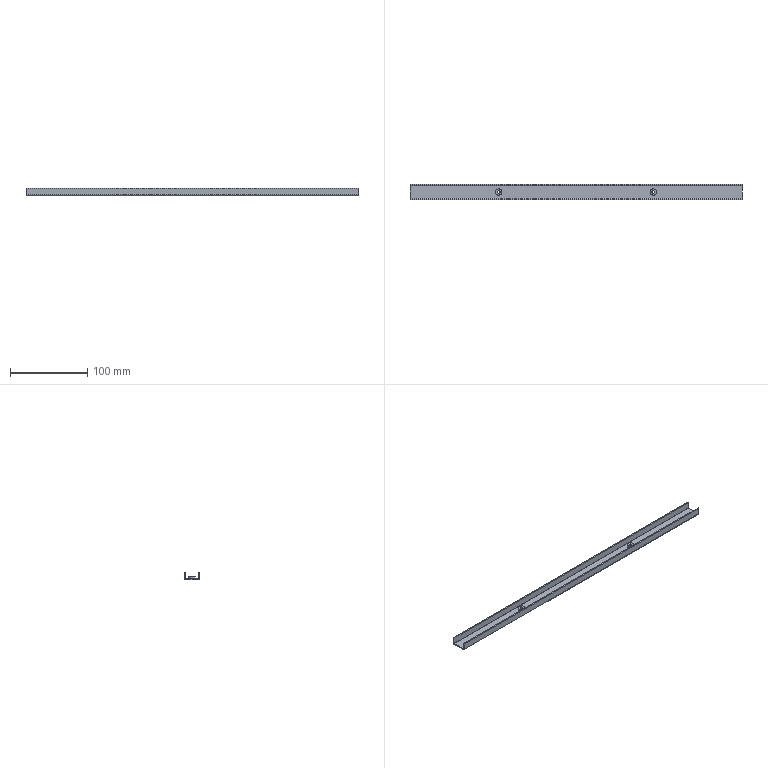Part | STEP file | FHD-021-014-C acrylic mounting strip | 1 solid | 20 faces | box 430 x 20 x 10 mm | volume 23632 mm3 | plane 12 | cylinder 8 | commonest cylinder face diameters 0.4 x2 3.3 x2 3.4 x2 8.3 x2
STEP:
#1=CARTESIAN_POINT('',(0.,0.,0.));
#2=DIRECTION('',(0.,0.,1.));
#3=DIRECTION('',(1.,0.,0.));
#4=AXIS2_PLACEMENT_3D('',#1,#2,#3);
#5=CARTESIAN_POINT('',(-215.,-8.3,-1.5));
#6=VERTEX_POINT('',#5);
#7=CARTESIAN_POINT('',(-215.,8.3,-1.5));
#8=VERTEX_POINT('',#7);
#9=CARTESIAN_POINT('',(-215.,0.,-1.5));
#10=DIRECTION('',(0.,1.,0.));
#11=VECTOR('',#10,1.);
#12=LINE('',#9,#11);
#13=CARTESIAN_POINT('',(0.,0.,-1.5));
#14=DIRECTION('',(0.,0.,-1.));
#15=DIRECTION('',(-1.,0.,0.));
#16=AXIS2_PLACEMENT_3D('',#13,#14,#15);
#17=PLANE('',#16);
#18=CARTESIAN_POINT('',(215.,0.));
#19=DIRECTION('',(0.,1.));
#20=VECTOR('',#19,1.);
#21=LINE('',#18,#20);
#22=(GEOMETRIC_REPRESENTATION_CONTEXT(2)PARAMETRIC_REPRESENTATION_CONTEXT()REPRESENTATION_CONTEXT('',''));
#23=DEFINITIONAL_REPRESENTATION('',(#21),#22);
#24=PCURVE('',#17,#23);
#25=CARTESIAN_POINT('',(-215.,-10.,-1.5));
#26=DIRECTION('',(-1.,0.,0.));
#27=DIRECTION('',(0.,0.,1.));
#28=AXIS2_PLACEMENT_3D('',#25,#26,#27);
#29=PLANE('',#28);
#30=CARTESIAN_POINT('',(0.,10.));
#31=DIRECTION('',(0.,1.));
#32=VECTOR('',#31,1.);
#33=LINE('',#30,#32);
#34=(GEOMETRIC_REPRESENTATION_CONTEXT(2)PARAMETRIC_REPRESENTATION_CONTEXT()REPRESENTATION_CONTEXT('',''));
#35=DEFINITIONAL_REPRESENTATION('',(#33),#34);
#36=PCURVE('',#29,#35);
#37=SURFACE_CURVE('',#12,(#24,#36),.PCURVE_S1.);
#38=EDGE_CURVE('',#6,#8,#37,.T.);
#39=ORIENTED_EDGE('',*,*,#38,.T.);
#40=CARTESIAN_POINT('',(215.,8.3,-1.5));
#41=VERTEX_POINT('',#40);
#42=CARTESIAN_POINT('',(0.,8.3,-1.5));
#43=DIRECTION('',(1.,0.,0.));
#44=VECTOR('',#43,1.);
#45=LINE('',#42,#44);
#46=CARTESIAN_POINT('',(0.,8.3));
#47=DIRECTION('',(-1.,0.));
#48=VECTOR('',#47,1.);
#49=LINE('',#46,#48);
#50=(GEOMETRIC_REPRESENTATION_CONTEXT(2)PARAMETRIC_REPRESENTATION_CONTEXT()REPRESENTATION_CONTEXT('',''));
#51=DEFINITIONAL_REPRESENTATION('',(#49),#50);
#52=PCURVE('',#17,#51);
#53=CARTESIAN_POINT('',(-215.,8.3,0.2));
#54=DIRECTION('',(-1.,0.,0.));
#55=DIRECTION('',(0.,0.,1.));
#56=AXIS2_PLACEMENT_3D('',#53,#54,#55);
#57=CYLINDRICAL_SURFACE('',#56,1.7);
#58=CARTESIAN_POINT('',(3.142,-215.));
#59=DIRECTION('',(0.,-1.));
#60=VECTOR('',#59,1.);
#61=LINE('',#58,#60);
#62=(GEOMETRIC_REPRESENTATION_CONTEXT(2)PARAMETRIC_REPRESENTATION_CONTEXT()REPRESENTATION_CONTEXT('',''));
#63=DEFINITIONAL_REPRESENTATION('',(#61),#62);
#64=PCURVE('',#57,#63);
#65=SURFACE_CURVE('',#45,(#52,#64),.PCURVE_S1.);
#66=EDGE_CURVE('',#8,#41,#65,.T.);
#67=ORIENTED_EDGE('',*,*,#66,.T.);
#68=CARTESIAN_POINT('',(215.,-8.3,-1.5));
#69=VERTEX_POINT('',#68);
#70=CARTESIAN_POINT('',(215.,0.,-1.5));
#71=DIRECTION('',(0.,-1.,0.));
#72=VECTOR('',#71,1.);
#73=LINE('',#70,#72);
#74=CARTESIAN_POINT('',(-215.,0.));
#75=DIRECTION('',(0.,-1.));
#76=VECTOR('',#75,1.);
#77=LINE('',#74,#76);
#78=(GEOMETRIC_REPRESENTATION_CONTEXT(2)PARAMETRIC_REPRESENTATION_CONTEXT()REPRESENTATION_CONTEXT('',''));
#79=DEFINITIONAL_REPRESENTATION('',(#77),#78);
#80=PCURVE('',#17,#79);
#81=CARTESIAN_POINT('',(215.,-10.,-1.5));
#82=DIRECTION('',(1.,0.,0.));
#83=DIRECTION('',(0.,0.,-1.));
#84=AXIS2_PLACEMENT_3D('',#81,#82,#83);
#85=PLANE('',#84);
#86=CARTESIAN_POINT('',(0.,10.));
#87=DIRECTION('',(0.,-1.));
#88=VECTOR('',#87,1.);
#89=LINE('',#86,#88);
#90=(GEOMETRIC_REPRESENTATION_CONTEXT(2)PARAMETRIC_REPRESENTATION_CONTEXT()REPRESENTATION_CONTEXT('',''));
#91=DEFINITIONAL_REPRESENTATION('',(#89),#90);
#92=PCURVE('',#85,#91);
#93=SURFACE_CURVE('',#73,(#80,#92),.PCURVE_S1.);
#94=EDGE_CURVE('',#41,#69,#93,.T.);
#95=ORIENTED_EDGE('',*,*,#94,.T.);
#96=CARTESIAN_POINT('',(0.,-8.3,-1.5));
#97=DIRECTION('',(-1.,0.,0.));
#98=VECTOR('',#97,1.);
#99=LINE('',#96,#98);
#100=CARTESIAN_POINT('',(0.,-8.3));
#101=DIRECTION('',(1.,0.));
#102=VECTOR('',#101,1.);
#103=LINE('',#100,#102);
#104=(GEOMETRIC_REPRESENTATION_CONTEXT(2)PARAMETRIC_REPRESENTATION_CONTEXT()REPRESENTATION_CONTEXT('',''));
#105=DEFINITIONAL_REPRESENTATION('',(#103),#104);
#106=PCURVE('',#17,#105);
#107=CARTESIAN_POINT('',(215.,-8.3,0.2));
#108=DIRECTION('',(1.,0.,0.));
#109=DIRECTION('',(0.,0.,-1.));
#110=AXIS2_PLACEMENT_3D('',#107,#108,#109);
#111=CYLINDRICAL_SURFACE('',#110,1.7);
#112=CARTESIAN_POINT('',(6.283,-215.));
#113=DIRECTION('',(0.,-1.));
#114=VECTOR('',#113,1.);
#115=LINE('',#112,#114);
#116=(GEOMETRIC_REPRESENTATION_CONTEXT(2)PARAMETRIC_REPRESENTATION_CONTEXT()REPRESENTATION_CONTEXT('',''));
#117=DEFINITIONAL_REPRESENTATION('',(#115),#116);
#118=PCURVE('',#111,#117);
#119=SURFACE_CURVE('',#99,(#106,#118),.PCURVE_S1.);
#120=EDGE_CURVE('',#69,#6,#119,.T.);
#121=ORIENTED_EDGE('',*,*,#120,.T.);
#122=EDGE_LOOP('',(#39,#67,#95,#121));
#123=FACE_BOUND('',#122,.T.);
#124=CARTESIAN_POINT('',(-101.65,0.,-1.5));
#125=VERTEX_POINT('',#124);
#126=CARTESIAN_POINT('',(-100.,0.,-1.5));
#127=DIRECTION('',(0.,0.,1.));
#128=DIRECTION('',(-1.,0.,0.));
#129=AXIS2_PLACEMENT_3D('',#126,#127,#128);
#130=CIRCLE('',#129,1.65);
#131=CARTESIAN_POINT('',(101.65,0.));
#132=CARTESIAN_POINT('',(101.65,-2.858));
#133=CARTESIAN_POINT('',(99.175,-1.429));
#134=CARTESIAN_POINT('',(96.7,0.));
#135=CARTESIAN_POINT('',(99.175,1.429));
#136=CARTESIAN_POINT('',(101.65,2.858));
#137=CARTESIAN_POINT('',(101.65,0.));
#138=(BOUNDED_CURVE()B_SPLINE_CURVE(2,(#131,#132,#133,#134,#135,#136,#137),.UNSPECIFIED.,.T.,.F.)B_SPLINE_CURVE_WITH_KNOTS((1,2,2,2,2,1),(-2.094,0.,2.094,4.189,6.283,8.378),.UNSPECIFIED.)CURVE()GEOMETRIC_REPRESENTATION_ITEM()RATIONAL_B_SPLINE_CURVE((1.,0.5,1.,0.5,1.,0.5,1.))REPRESENTATION_ITEM(''));
#139=(GEOMETRIC_REPRESENTATION_CONTEXT(2)PARAMETRIC_REPRESENTATION_CONTEXT()REPRESENTATION_CONTEXT('',''));
#140=DEFINITIONAL_REPRESENTATION('',(#138),#139);
#141=PCURVE('',#17,#140);
#142=CARTESIAN_POINT('',(-100.,0.,-1.5));
#143=DIRECTION('',(0.,0.,-1.));
#144=DIRECTION('',(-1.,0.,0.));
#145=AXIS2_PLACEMENT_3D('',#142,#143,#144);
#146=CYLINDRICAL_SURFACE('',#145,1.65);
#147=CARTESIAN_POINT('',(6.283,0.));
#148=DIRECTION('',(-1.,0.));
#149=VECTOR('',#148,1.);
#150=LINE('',#147,#149);
#151=(GEOMETRIC_REPRESENTATION_CONTEXT(2)PARAMETRIC_REPRESENTATION_CONTEXT()REPRESENTATION_CONTEXT('',''));
#152=DEFINITIONAL_REPRESENTATION('',(#150),#151);
#153=PCURVE('',#146,#152);
#154=SURFACE_CURVE('',#130,(#141,#153),.PCURVE_S1.);
#155=EDGE_CURVE('',#125,#125,#154,.T.);
#156=ORIENTED_EDGE('',*,*,#155,.T.);
#157=EDGE_LOOP('',(#156));
#158=FACE_BOUND('',#157,.T.);
#159=CARTESIAN_POINT('',(98.35,0.,-1.5));
#160=VERTEX_POINT('',#159);
#161=CARTESIAN_POINT('',(100.,0.,-1.5));
#162=DIRECTION('',(0.,0.,1.));
#163=DIRECTION('',(-1.,0.,0.));
#164=AXIS2_PLACEMENT_3D('',#161,#162,#163);
#165=CIRCLE('',#164,1.65);
#166=CARTESIAN_POINT('',(-98.35,0.));
#167=CARTESIAN_POINT('',(-98.35,-2.858));
#168=CARTESIAN_POINT('',(-100.825,-1.429));
#169=CARTESIAN_POINT('',(-103.3,0.));
#170=CARTESIAN_POINT('',(-100.825,1.429));
#171=CARTESIAN_POINT('',(-98.35,2.858));
#172=CARTESIAN_POINT('',(-98.35,0.));
#173=(BOUNDED_CURVE()B_SPLINE_CURVE(2,(#166,#167,#168,#169,#170,#171,#172),.UNSPECIFIED.,.T.,.F.)B_SPLINE_CURVE_WITH_KNOTS((1,2,2,2,2,1),(-2.094,0.,2.094,4.189,6.283,8.378),.UNSPECIFIED.)CURVE()GEOMETRIC_REPRESENTATION_ITEM()RATIONAL_B_SPLINE_CURVE((1.,0.5,1.,0.5,1.,0.5,1.))REPRESENTATION_ITEM(''));
#174=(GEOMETRIC_REPRESENTATION_CONTEXT(2)PARAMETRIC_REPRESENTATION_CONTEXT()REPRESENTATION_CONTEXT('',''));
#175=DEFINITIONAL_REPRESENTATION('',(#173),#174);
#176=PCURVE('',#17,#175);
#177=CARTESIAN_POINT('',(100.,0.,-1.5));
#178=DIRECTION('',(0.,0.,-1.));
#179=DIRECTION('',(-1.,0.,0.));
#180=AXIS2_PLACEMENT_3D('',#177,#178,#179);
#181=CYLINDRICAL_SURFACE('',#180,1.65);
#182=CARTESIAN_POINT('',(6.283,0.));
#183=DIRECTION('',(-1.,0.));
#184=VECTOR('',#183,1.);
#185=LINE('',#182,#184);
#186=(GEOMETRIC_REPRESENTATION_CONTEXT(2)PARAMETRIC_REPRESENTATION_CONTEXT()REPRESENTATION_CONTEXT('',''));
#187=DEFINITIONAL_REPRESENTATION('',(#185),#186);
#188=PCURVE('',#181,#187);
#189=SURFACE_CURVE('',#165,(#176,#188),.PCURVE_S1.);
#190=EDGE_CURVE('',#160,#160,#189,.T.);
#191=ORIENTED_EDGE('',*,*,#190,.T.);
#192=EDGE_LOOP('',(#191));
#193=FACE_BOUND('',#192,.T.);
#194=ADVANCED_FACE('',(#123,#158,#193),#17,.T.);
#195=CARTESIAN_POINT('',(-215.,10.,0.2));
#196=VERTEX_POINT('',#195);
#197=CARTESIAN_POINT('',(215.,10.,0.2));
#198=VERTEX_POINT('',#197);
#199=CARTESIAN_POINT('',(-215.,10.,0.2));
#200=DIRECTION('',(1.,0.,0.));
#201=VECTOR('',#200,1.);
#202=LINE('',#199,#201);
#203=CARTESIAN_POINT('',(1.571,0.));
#204=DIRECTION('',(0.,-1.));
#205=VECTOR('',#204,1.);
#206=LINE('',#203,#205);
#207=(GEOMETRIC_REPRESENTATION_CONTEXT(2)PARAMETRIC_REPRESENTATION_CONTEXT()REPRESENTATION_CONTEXT('',''));
#208=DEFINITIONAL_REPRESENTATION('',(#206),#207);
#209=PCURVE('',#57,#208);
#210=CARTESIAN_POINT('',(0.,10.,0.));
#211=DIRECTION('',(0.,-1.,0.));
#212=DIRECTION('',(0.,0.,-1.));
#213=AXIS2_PLACEMENT_3D('',#210,#211,#212);
#214=PLANE('',#213);
#215=CARTESIAN_POINT('',(-0.2,-215.));
#216=DIRECTION('',(0.,1.));
#217=VECTOR('',#216,1.);
#218=LINE('',#215,#217);
#219=(GEOMETRIC_REPRESENTATION_CONTEXT(2)PARAMETRIC_REPRESENTATION_CONTEXT()REPRESENTATION_CONTEXT('',''));
#220=DEFINITIONAL_REPRESENTATION('',(#218),#219);
#221=PCURVE('',#214,#220);
#222=SURFACE_CURVE('',#202,(#209,#221),.PCURVE_S1.);
#223=EDGE_CURVE('',#196,#198,#222,.T.);
#224=ORIENTED_EDGE('',*,*,#223,.T.);
#225=CARTESIAN_POINT('',(215.,8.3,0.2));
#226=DIRECTION('',(-1.,0.,0.));
#227=DIRECTION('',(0.,0.,1.));
#228=AXIS2_PLACEMENT_3D('',#225,#226,#227);
#229=CIRCLE('',#228,1.7);
#230=CARTESIAN_POINT('',(0.,-430.));
#231=DIRECTION('',(1.,0.));
#232=VECTOR('',#231,1.);
#233=LINE('',#230,#232);
#234=(GEOMETRIC_REPRESENTATION_CONTEXT(2)PARAMETRIC_REPRESENTATION_CONTEXT()REPRESENTATION_CONTEXT('',''));
#235=DEFINITIONAL_REPRESENTATION('',(#233),#234);
#236=PCURVE('',#57,#235);
#237=CARTESIAN_POINT('',(-3.4,18.3));
#238=CARTESIAN_POINT('',(-3.4,21.244));
#239=CARTESIAN_POINT('',(-0.85,19.772));
#240=CARTESIAN_POINT('',(1.7,18.3));
#241=CARTESIAN_POINT('',(-0.85,16.828));
#242=CARTESIAN_POINT('',(-3.4,15.356));
#243=CARTESIAN_POINT('',(-3.4,18.3));
#244=(BOUNDED_CURVE()B_SPLINE_CURVE(2,(#237,#238,#239,#240,#241,#242,#243),.UNSPECIFIED.,.T.,.F.)B_SPLINE_CURVE_WITH_KNOTS((1,2,2,2,2,1),(-2.094,0.,2.094,4.189,6.283,8.378),.UNSPECIFIED.)CURVE()GEOMETRIC_REPRESENTATION_ITEM()RATIONAL_B_SPLINE_CURVE((1.,0.5,1.,0.5,1.,0.5,1.))REPRESENTATION_ITEM(''));
#245=(GEOMETRIC_REPRESENTATION_CONTEXT(2)PARAMETRIC_REPRESENTATION_CONTEXT()REPRESENTATION_CONTEXT('',''));
#246=DEFINITIONAL_REPRESENTATION('',(#244),#245);
#247=PCURVE('',#85,#246);
#248=SURFACE_CURVE('',#229,(#236,#247),.PCURVE_S1.);
#249=EDGE_CURVE('',#198,#41,#248,.T.);
#250=ORIENTED_EDGE('',*,*,#249,.T.);
#251=ORIENTED_EDGE('',*,*,#66,.F.);
#252=CARTESIAN_POINT('',(-215.,8.3,0.2));
#253=DIRECTION('',(1.,0.,0.));
#254=DIRECTION('',(0.,0.,1.));
#255=AXIS2_PLACEMENT_3D('',#252,#253,#254);
#256=CIRCLE('',#255,1.7);
#257=CARTESIAN_POINT('',(6.283,0.));
#258=DIRECTION('',(-1.,0.));
#259=VECTOR('',#258,1.);
#260=LINE('',#257,#259);
#261=(GEOMETRIC_REPRESENTATION_CONTEXT(2)PARAMETRIC_REPRESENTATION_CONTEXT()REPRESENTATION_CONTEXT('',''));
#262=DEFINITIONAL_REPRESENTATION('',(#260),#261);
#263=PCURVE('',#57,#262);
#264=CARTESIAN_POINT('',(3.4,18.3));
#265=CARTESIAN_POINT('',(3.4,15.356));
#266=CARTESIAN_POINT('',(0.85,16.828));
#267=CARTESIAN_POINT('',(-1.7,18.3));
#268=CARTESIAN_POINT('',(0.85,19.772));
#269=CARTESIAN_POINT('',(3.4,21.244));
#270=CARTESIAN_POINT('',(3.4,18.3));
#271=(BOUNDED_CURVE()B_SPLINE_CURVE(2,(#264,#265,#266,#267,#268,#269,#270),.UNSPECIFIED.,.T.,.F.)B_SPLINE_CURVE_WITH_KNOTS((1,2,2,2,2,1),(-2.094,0.,2.094,4.189,6.283,8.378),.UNSPECIFIED.)CURVE()GEOMETRIC_REPRESENTATION_ITEM()RATIONAL_B_SPLINE_CURVE((1.,0.5,1.,0.5,1.,0.5,1.))REPRESENTATION_ITEM(''));
#272=(GEOMETRIC_REPRESENTATION_CONTEXT(2)PARAMETRIC_REPRESENTATION_CONTEXT()REPRESENTATION_CONTEXT('',''));
#273=DEFINITIONAL_REPRESENTATION('',(#271),#272);
#274=PCURVE('',#29,#273);
#275=SURFACE_CURVE('',#256,(#263,#274),.PCURVE_S1.);
#276=EDGE_CURVE('',#8,#196,#275,.T.);
#277=ORIENTED_EDGE('',*,*,#276,.T.);
#278=EDGE_LOOP('',(#224,#250,#251,#277));
#279=FACE_BOUND('',#278,.T.);
#280=ADVANCED_FACE('',(#279),#57,.T.);
#281=CARTESIAN_POINT('',(-215.,-8.3,0.));
#282=VERTEX_POINT('',#281);
#283=CARTESIAN_POINT('',(-215.,8.3,0.));
#284=VERTEX_POINT('',#283);
#285=CARTESIAN_POINT('',(-215.,-10.,0.));
#286=DIRECTION('',(0.,1.,0.));
#287=VECTOR('',#286,1.);
#288=LINE('',#285,#287);
#289=CARTESIAN_POINT('',(1.5,0.));
#290=DIRECTION('',(0.,1.));
#291=VECTOR('',#290,1.);
#292=LINE('',#289,#291);
#293=(GEOMETRIC_REPRESENTATION_CONTEXT(2)PARAMETRIC_REPRESENTATION_CONTEXT()REPRESENTATION_CONTEXT('',''));
#294=DEFINITIONAL_REPRESENTATION('',(#292),#293);
#295=PCURVE('',#29,#294);
#296=CARTESIAN_POINT('',(0.,0.,0.));
#297=DIRECTION('',(0.,0.,-1.));
#298=DIRECTION('',(-1.,0.,0.));
#299=AXIS2_PLACEMENT_3D('',#296,#297,#298);
#300=PLANE('',#299);
#301=CARTESIAN_POINT('',(215.,-10.));
#302=DIRECTION('',(0.,1.));
#303=VECTOR('',#302,1.);
#304=LINE('',#301,#303);
#305=(GEOMETRIC_REPRESENTATION_CONTEXT(2)PARAMETRIC_REPRESENTATION_CONTEXT()REPRESENTATION_CONTEXT('',''));
#306=DEFINITIONAL_REPRESENTATION('',(#304),#305);
#307=PCURVE('',#300,#306);
#308=SURFACE_CURVE('',#288,(#295,#307),.PCURVE_S1.);
#309=EDGE_CURVE('',#282,#284,#308,.T.);
#310=ORIENTED_EDGE('',*,*,#309,.T.);
#311=CARTESIAN_POINT('',(-215.,8.5,0.2));
#312=VERTEX_POINT('',#311);
#313=CARTESIAN_POINT('',(-215.,8.3,0.2));
#314=DIRECTION('',(1.,0.,0.));
#315=DIRECTION('',(0.,0.,1.));
#316=AXIS2_PLACEMENT_3D('',#313,#314,#315);
#317=CIRCLE('',#316,0.2);
#318=CARTESIAN_POINT('',(1.9,18.3));
#319=CARTESIAN_POINT('',(1.9,17.954));
#320=CARTESIAN_POINT('',(1.6,18.127));
#321=CARTESIAN_POINT('',(1.3,18.3));
#322=CARTESIAN_POINT('',(1.6,18.473));
#323=CARTESIAN_POINT('',(1.9,18.646));
#324=CARTESIAN_POINT('',(1.9,18.3));
#325=(BOUNDED_CURVE()B_SPLINE_CURVE(2,(#318,#319,#320,#321,#322,#323,#324),.UNSPECIFIED.,.T.,.F.)B_SPLINE_CURVE_WITH_KNOTS((1,2,2,2,2,1),(-2.094,0.,2.094,4.189,6.283,8.378),.UNSPECIFIED.)CURVE()GEOMETRIC_REPRESENTATION_ITEM()RATIONAL_B_SPLINE_CURVE((1.,0.5,1.,0.5,1.,0.5,1.))REPRESENTATION_ITEM(''));
#326=(GEOMETRIC_REPRESENTATION_CONTEXT(2)PARAMETRIC_REPRESENTATION_CONTEXT()REPRESENTATION_CONTEXT('',''));
#327=DEFINITIONAL_REPRESENTATION('',(#325),#326);
#328=PCURVE('',#29,#327);
#329=CARTESIAN_POINT('',(-215.,8.3,0.2));
#330=DIRECTION('',(-1.,0.,0.));
#331=DIRECTION('',(0.,0.,1.));
#332=AXIS2_PLACEMENT_3D('',#329,#330,#331);
#333=CYLINDRICAL_SURFACE('',#332,0.2);
#334=CARTESIAN_POINT('',(6.283,0.));
#335=DIRECTION('',(-1.,0.));
#336=VECTOR('',#335,1.);
#337=LINE('',#334,#336);
#338=(GEOMETRIC_REPRESENTATION_CONTEXT(2)PARAMETRIC_REPRESENTATION_CONTEXT()REPRESENTATION_CONTEXT('',''));
#339=DEFINITIONAL_REPRESENTATION('',(#337),#338);
#340=PCURVE('',#333,#339);
#341=SURFACE_CURVE('',#317,(#328,#340),.PCURVE_S1.);
#342=EDGE_CURVE('',#284,#312,#341,.T.);
#343=ORIENTED_EDGE('',*,*,#342,.T.);
#344=CARTESIAN_POINT('',(-215.,8.5,8.5));
#345=VERTEX_POINT('',#344);
#346=CARTESIAN_POINT('',(-215.,8.5,8.5));
#347=DIRECTION('',(0.,0.,-1.));
#348=VECTOR('',#347,1.);
#349=LINE('',#346,#348);
#350=CARTESIAN_POINT('',(10.,18.5));
#351=DIRECTION('',(-1.,0.));
#352=VECTOR('',#351,1.);
#353=LINE('',#350,#352);
#354=(GEOMETRIC_REPRESENTATION_CONTEXT(2)PARAMETRIC_REPRESENTATION_CONTEXT()REPRESENTATION_CONTEXT('',''));
#355=DEFINITIONAL_REPRESENTATION('',(#353),#354);
#356=PCURVE('',#29,#355);
#357=CARTESIAN_POINT('',(0.,8.5,0.));
#358=DIRECTION('',(0.,-1.,0.));
#359=DIRECTION('',(0.,0.,-1.));
#360=AXIS2_PLACEMENT_3D('',#357,#358,#359);
#361=PLANE('',#360);
#362=CARTESIAN_POINT('',(-8.5,-215.));
#363=DIRECTION('',(1.,0.));
#364=VECTOR('',#363,1.);
#365=LINE('',#362,#364);
#366=(GEOMETRIC_REPRESENTATION_CONTEXT(2)PARAMETRIC_REPRESENTATION_CONTEXT()REPRESENTATION_CONTEXT('',''));
#367=DEFINITIONAL_REPRESENTATION('',(#365),#366);
#368=PCURVE('',#361,#367);
#369=SURFACE_CURVE('',#349,(#356,#368),.PCURVE_S1.);
#370=EDGE_CURVE('',#345,#312,#369,.T.);
#371=ORIENTED_EDGE('',*,*,#370,.F.);
#372=CARTESIAN_POINT('',(-215.,10.,8.5));
#373=VERTEX_POINT('',#372);
#374=CARTESIAN_POINT('',(-215.,10.,8.5));
#375=DIRECTION('',(0.,-1.,0.));
#376=VECTOR('',#375,1.);
#377=LINE('',#374,#376);
#378=CARTESIAN_POINT('',(10.,20.));
#379=DIRECTION('',(0.,-1.));
#380=VECTOR('',#379,1.);
#381=LINE('',#378,#380);
#382=(GEOMETRIC_REPRESENTATION_CONTEXT(2)PARAMETRIC_REPRESENTATION_CONTEXT()REPRESENTATION_CONTEXT('',''));
#383=DEFINITIONAL_REPRESENTATION('',(#381),#382);
#384=PCURVE('',#29,#383);
#385=CARTESIAN_POINT('',(215.,10.,8.5));
#386=DIRECTION('',(0.,0.,-1.));
#387=DIRECTION('',(0.,1.,0.));
#388=AXIS2_PLACEMENT_3D('',#385,#386,#387);
#389=PLANE('',#388);
#390=CARTESIAN_POINT('',(0.,-430.));
#391=DIRECTION('',(-1.,0.));
#392=VECTOR('',#391,1.);
#393=LINE('',#390,#392);
#394=(GEOMETRIC_REPRESENTATION_CONTEXT(2)PARAMETRIC_REPRESENTATION_CONTEXT()REPRESENTATION_CONTEXT('',''));
#395=DEFINITIONAL_REPRESENTATION('',(#393),#394);
#396=PCURVE('',#389,#395);
#397=SURFACE_CURVE('',#377,(#384,#396),.PCURVE_S1.);
#398=EDGE_CURVE('',#373,#345,#397,.T.);
#399=ORIENTED_EDGE('',*,*,#398,.F.);
#400=CARTESIAN_POINT('',(-215.,10.,0.));
#401=DIRECTION('',(0.,0.,-1.));
#402=VECTOR('',#401,1.);
#403=LINE('',#400,#402);
#404=CARTESIAN_POINT('',(1.5,20.));
#405=DIRECTION('',(-1.,0.));
#406=VECTOR('',#405,1.);
#407=LINE('',#404,#406);
#408=(GEOMETRIC_REPRESENTATION_CONTEXT(2)PARAMETRIC_REPRESENTATION_CONTEXT()REPRESENTATION_CONTEXT('',''));
#409=DEFINITIONAL_REPRESENTATION('',(#407),#408);
#410=PCURVE('',#29,#409);
#411=CARTESIAN_POINT('',(0.,-215.));
#412=DIRECTION('',(1.,0.));
#413=VECTOR('',#412,1.);
#414=LINE('',#411,#413);
#415=(GEOMETRIC_REPRESENTATION_CONTEXT(2)PARAMETRIC_REPRESENTATION_CONTEXT()REPRESENTATION_CONTEXT('',''));
#416=DEFINITIONAL_REPRESENTATION('',(#414),#415);
#417=PCURVE('',#214,#416);
#418=SURFACE_CURVE('',#403,(#410,#417),.PCURVE_S1.);
#419=EDGE_CURVE('',#373,#196,#418,.T.);
#420=ORIENTED_EDGE('',*,*,#419,.T.);
#421=ORIENTED_EDGE('',*,*,#276,.F.);
#422=ORIENTED_EDGE('',*,*,#38,.F.);
#423=CARTESIAN_POINT('',(-215.,-10.,0.2));
#424=VERTEX_POINT('',#423);
#425=CARTESIAN_POINT('',(-215.,-8.3,0.2));
#426=DIRECTION('',(1.,0.,0.));
#427=DIRECTION('',(0.,0.,-1.));
#428=AXIS2_PLACEMENT_3D('',#425,#426,#427);
#429=CIRCLE('',#428,1.7);
#430=CARTESIAN_POINT('',(0.,1.7));
#431=CARTESIAN_POINT('',(0.,4.644));
#432=CARTESIAN_POINT('',(2.55,3.172));
#433=CARTESIAN_POINT('',(5.1,1.7));
#434=CARTESIAN_POINT('',(2.55,0.2278));
#435=CARTESIAN_POINT('',(0.,-1.244));
#436=CARTESIAN_POINT('',(0.,1.7));
#437=(BOUNDED_CURVE()B_SPLINE_CURVE(2,(#430,#431,#432,#433,#434,#435,#436),.UNSPECIFIED.,.T.,.F.)B_SPLINE_CURVE_WITH_KNOTS((1,2,2,2,2,1),(-2.094,0.,2.094,4.189,6.283,8.378),.UNSPECIFIED.)CURVE()GEOMETRIC_REPRESENTATION_ITEM()RATIONAL_B_SPLINE_CURVE((1.,0.5,1.,0.5,1.,0.5,1.))REPRESENTATION_ITEM(''));
#438=(GEOMETRIC_REPRESENTATION_CONTEXT(2)PARAMETRIC_REPRESENTATION_CONTEXT()REPRESENTATION_CONTEXT('',''));
#439=DEFINITIONAL_REPRESENTATION('',(#437),#438);
#440=PCURVE('',#29,#439);
#441=CARTESIAN_POINT('',(0.,-430.));
#442=DIRECTION('',(1.,0.));
#443=VECTOR('',#442,1.);
#444=LINE('',#441,#443);
#445=(GEOMETRIC_REPRESENTATION_CONTEXT(2)PARAMETRIC_REPRESENTATION_CONTEXT()REPRESENTATION_CONTEXT('',''));
#446=DEFINITIONAL_REPRESENTATION('',(#444),#445);
#447=PCURVE('',#111,#446);
#448=SURFACE_CURVE('',#429,(#440,#447),.PCURVE_S1.);
#449=EDGE_CURVE('',#424,#6,#448,.T.);
#450=ORIENTED_EDGE('',*,*,#449,.F.);
#451=CARTESIAN_POINT('',(-215.,-10.,8.5));
#452=VERTEX_POINT('',#451);
#453=CARTESIAN_POINT('',(-215.,-10.,0.));
#454=DIRECTION('',(0.,0.,1.));
#455=VECTOR('',#454,1.);
#456=LINE('',#453,#455);
#457=CARTESIAN_POINT('',(1.5,0.));
#458=DIRECTION('',(1.,0.));
#459=VECTOR('',#458,1.);
#460=LINE('',#457,#459);
#461=(GEOMETRIC_REPRESENTATION_CONTEXT(2)PARAMETRIC_REPRESENTATION_CONTEXT()REPRESENTATION_CONTEXT('',''));
#462=DEFINITIONAL_REPRESENTATION('',(#460),#461);
#463=PCURVE('',#29,#462);
#464=CARTESIAN_POINT('',(0.,-10.,0.));
#465=DIRECTION('',(0.,1.,0.));
#466=DIRECTION('',(0.,0.,1.));
#467=AXIS2_PLACEMENT_3D('',#464,#465,#466);
#468=PLANE('',#467);
#469=CARTESIAN_POINT('',(0.,-215.));
#470=DIRECTION('',(1.,0.));
#471=VECTOR('',#470,1.);
#472=LINE('',#469,#471);
#473=(GEOMETRIC_REPRESENTATION_CONTEXT(2)PARAMETRIC_REPRESENTATION_CONTEXT()REPRESENTATION_CONTEXT('',''));
#474=DEFINITIONAL_REPRESENTATION('',(#472),#473);
#475=PCURVE('',#468,#474);
#476=SURFACE_CURVE('',#456,(#463,#475),.PCURVE_S1.);
#477=EDGE_CURVE('',#424,#452,#476,.T.);
#478=ORIENTED_EDGE('',*,*,#477,.T.);
#479=CARTESIAN_POINT('',(-215.,-8.5,8.5));
#480=VERTEX_POINT('',#479);
#481=CARTESIAN_POINT('',(-215.,-10.,8.5));
#482=DIRECTION('',(0.,1.,0.));
#483=VECTOR('',#482,1.);
#484=LINE('',#481,#483);
#485=CARTESIAN_POINT('',(10.,0.));
#486=DIRECTION('',(0.,1.));
#487=VECTOR('',#486,1.);
#488=LINE('',#485,#487);
#489=(GEOMETRIC_REPRESENTATION_CONTEXT(2)PARAMETRIC_REPRESENTATION_CONTEXT()REPRESENTATION_CONTEXT('',''));
#490=DEFINITIONAL_REPRESENTATION('',(#488),#489);
#491=PCURVE('',#29,#490);
#492=CARTESIAN_POINT('',(-215.,-10.,8.5));
#493=DIRECTION('',(0.,0.,-1.));
#494=DIRECTION('',(0.,1.,0.));
#495=AXIS2_PLACEMENT_3D('',#492,#493,#494);
#496=PLANE('',#495);
#497=CARTESIAN_POINT('',(0.,0.));
#498=DIRECTION('',(1.,0.));
#499=VECTOR('',#498,1.);
#500=LINE('',#497,#499);
#501=(GEOMETRIC_REPRESENTATION_CONTEXT(2)PARAMETRIC_REPRESENTATION_CONTEXT()REPRESENTATION_CONTEXT('',''));
#502=DEFINITIONAL_REPRESENTATION('',(#500),#501);
#503=PCURVE('',#496,#502);
#504=SURFACE_CURVE('',#484,(#491,#503),.PCURVE_S1.);
#505=EDGE_CURVE('',#452,#480,#504,.T.);
#506=ORIENTED_EDGE('',*,*,#505,.T.);
#507=CARTESIAN_POINT('',(-215.,-8.5,0.2));
#508=VERTEX_POINT('',#507);
#509=CARTESIAN_POINT('',(-215.,-8.5,0.));
#510=DIRECTION('',(0.,0.,1.));
#511=VECTOR('',#510,1.);
#512=LINE('',#509,#511);
#513=CARTESIAN_POINT('',(1.5,1.5));
#514=DIRECTION('',(1.,0.));
#515=VECTOR('',#514,1.);
#516=LINE('',#513,#515);
#517=(GEOMETRIC_REPRESENTATION_CONTEXT(2)PARAMETRIC_REPRESENTATION_CONTEXT()REPRESENTATION_CONTEXT('',''));
#518=DEFINITIONAL_REPRESENTATION('',(#516),#517);
#519=PCURVE('',#29,#518);
#520=CARTESIAN_POINT('',(0.,-8.5,0.));
#521=DIRECTION('',(0.,1.,0.));
#522=DIRECTION('',(0.,0.,1.));
#523=AXIS2_PLACEMENT_3D('',#520,#521,#522);
#524=PLANE('',#523);
#525=CARTESIAN_POINT('',(0.,-215.));
#526=DIRECTION('',(1.,0.));
#527=VECTOR('',#526,1.);
#528=LINE('',#525,#527);
#529=(GEOMETRIC_REPRESENTATION_CONTEXT(2)PARAMETRIC_REPRESENTATION_CONTEXT()REPRESENTATION_CONTEXT('',''));
#530=DEFINITIONAL_REPRESENTATION('',(#528),#529);
#531=PCURVE('',#524,#530);
#532=SURFACE_CURVE('',#512,(#519,#531),.PCURVE_S1.);
#533=EDGE_CURVE('',#508,#480,#532,.T.);
#534=ORIENTED_EDGE('',*,*,#533,.F.);
#535=CARTESIAN_POINT('',(-215.,-8.3,0.2));
#536=DIRECTION('',(1.,0.,0.));
#537=DIRECTION('',(0.,0.,-1.));
#538=AXIS2_PLACEMENT_3D('',#535,#536,#537);
#539=CIRCLE('',#538,0.2);
#540=CARTESIAN_POINT('',(1.5,1.7));
#541=CARTESIAN_POINT('',(1.5,2.046));
#542=CARTESIAN_POINT('',(1.8,1.873));
#543=CARTESIAN_POINT('',(2.1,1.7));
#544=CARTESIAN_POINT('',(1.8,1.527));
#545=CARTESIAN_POINT('',(1.5,1.354));
#546=CARTESIAN_POINT('',(1.5,1.7));
#547=(BOUNDED_CURVE()B_SPLINE_CURVE(2,(#540,#541,#542,#543,#544,#545,#546),.UNSPECIFIED.,.T.,.F.)B_SPLINE_CURVE_WITH_KNOTS((1,2,2,2,2,1),(-2.094,0.,2.094,4.189,6.283,8.378),.UNSPECIFIED.)CURVE()GEOMETRIC_REPRESENTATION_ITEM()RATIONAL_B_SPLINE_CURVE((1.,0.5,1.,0.5,1.,0.5,1.))REPRESENTATION_ITEM(''));
#548=(GEOMETRIC_REPRESENTATION_CONTEXT(2)PARAMETRIC_REPRESENTATION_CONTEXT()REPRESENTATION_CONTEXT('',''));
#549=DEFINITIONAL_REPRESENTATION('',(#547),#548);
#550=PCURVE('',#29,#549);
#551=CARTESIAN_POINT('',(215.,-8.3,0.2));
#552=DIRECTION('',(1.,0.,0.));
#553=DIRECTION('',(0.,0.,-1.));
#554=AXIS2_PLACEMENT_3D('',#551,#552,#553);
#555=CYLINDRICAL_SURFACE('',#554,0.2);
#556=CARTESIAN_POINT('',(0.,-430.));
#557=DIRECTION('',(1.,0.));
#558=VECTOR('',#557,1.);
#559=LINE('',#556,#558);
#560=(GEOMETRIC_REPRESENTATION_CONTEXT(2)PARAMETRIC_REPRESENTATION_CONTEXT()REPRESENTATION_CONTEXT('',''));
#561=DEFINITIONAL_REPRESENTATION('',(#559),#560);
#562=PCURVE('',#555,#561);
#563=SURFACE_CURVE('',#539,(#550,#562),.PCURVE_S1.);
#564=EDGE_CURVE('',#508,#282,#563,.T.);
#565=ORIENTED_EDGE('',*,*,#564,.T.);
#566=EDGE_LOOP('',(#310,#343,#371,#399,#420,#421,#422,#450,#478,#506,#534,#565));
#567=FACE_BOUND('',#566,.T.);
#568=ADVANCED_FACE('',(#567),#29,.T.);
#569=CARTESIAN_POINT('',(215.,-10.,0.2));
#570=VERTEX_POINT('',#569);
#571=CARTESIAN_POINT('',(215.,-10.,0.2));
#572=DIRECTION('',(-1.,0.,0.));
#573=VECTOR('',#572,1.);
#574=LINE('',#571,#573);
#575=CARTESIAN_POINT('',(4.712,0.));
#576=DIRECTION('',(0.,-1.));
#577=VECTOR('',#576,1.);
#578=LINE('',#575,#577);
#579=(GEOMETRIC_REPRESENTATION_CONTEXT(2)PARAMETRIC_REPRESENTATION_CONTEXT()REPRESENTATION_CONTEXT('',''));
#580=DEFINITIONAL_REPRESENTATION('',(#578),#579);
#581=PCURVE('',#111,#580);
#582=CARTESIAN_POINT('',(0.2,215.));
#583=DIRECTION('',(0.,-1.));
#584=VECTOR('',#583,1.);
#585=LINE('',#582,#584);
#586=(GEOMETRIC_REPRESENTATION_CONTEXT(2)PARAMETRIC_REPRESENTATION_CONTEXT()REPRESENTATION_CONTEXT('',''));
#587=DEFINITIONAL_REPRESENTATION('',(#585),#586);
#588=PCURVE('',#468,#587);
#589=SURFACE_CURVE('',#574,(#581,#588),.PCURVE_S1.);
#590=EDGE_CURVE('',#570,#424,#589,.T.);
#591=ORIENTED_EDGE('',*,*,#590,.T.);
#592=ORIENTED_EDGE('',*,*,#449,.T.);
#593=ORIENTED_EDGE('',*,*,#120,.F.);
#594=CARTESIAN_POINT('',(215.,-8.3,0.2));
#595=DIRECTION('',(-1.,0.,0.));
#596=DIRECTION('',(0.,0.,-1.));
#597=AXIS2_PLACEMENT_3D('',#594,#595,#596);
#598=CIRCLE('',#597,1.7);
#599=CARTESIAN_POINT('',(6.283,0.));
#600=DIRECTION('',(-1.,0.));
#601=VECTOR('',#600,1.);
#602=LINE('',#599,#601);
#603=(GEOMETRIC_REPRESENTATION_CONTEXT(2)PARAMETRIC_REPRESENTATION_CONTEXT()REPRESENTATION_CONTEXT('',''));
#604=DEFINITIONAL_REPRESENTATION('',(#602),#603);
#605=PCURVE('',#111,#604);
#606=CARTESIAN_POINT('',(0.,1.7));
#607=CARTESIAN_POINT('',(0.,-1.244));
#608=CARTESIAN_POINT('',(-2.55,0.2278));
#609=CARTESIAN_POINT('',(-5.1,1.7));
#610=CARTESIAN_POINT('',(-2.55,3.172));
#611=CARTESIAN_POINT('',(0.,4.644));
#612=CARTESIAN_POINT('',(0.,1.7));
#613=(BOUNDED_CURVE()B_SPLINE_CURVE(2,(#606,#607,#608,#609,#610,#611,#612),.UNSPECIFIED.,.T.,.F.)B_SPLINE_CURVE_WITH_KNOTS((1,2,2,2,2,1),(-2.094,0.,2.094,4.189,6.283,8.378),.UNSPECIFIED.)CURVE()GEOMETRIC_REPRESENTATION_ITEM()RATIONAL_B_SPLINE_CURVE((1.,0.5,1.,0.5,1.,0.5,1.))REPRESENTATION_ITEM(''));
#614=(GEOMETRIC_REPRESENTATION_CONTEXT(2)PARAMETRIC_REPRESENTATION_CONTEXT()REPRESENTATION_CONTEXT('',''));
#615=DEFINITIONAL_REPRESENTATION('',(#613),#614);
#616=PCURVE('',#85,#615);
#617=SURFACE_CURVE('',#598,(#605,#616),.PCURVE_S1.);
#618=EDGE_CURVE('',#69,#570,#617,.T.);
#619=ORIENTED_EDGE('',*,*,#618,.T.);
#620=EDGE_LOOP('',(#591,#592,#593,#619));
#621=FACE_BOUND('',#620,.T.);
#622=ADVANCED_FACE('',(#621),#111,.T.);
#623=ORIENTED_EDGE('',*,*,#94,.F.);
#624=ORIENTED_EDGE('',*,*,#249,.F.);
#625=CARTESIAN_POINT('',(215.,10.,8.5));
#626=VERTEX_POINT('',#625);
#627=CARTESIAN_POINT('',(215.,10.,0.));
#628=DIRECTION('',(0.,0.,1.));
#629=VECTOR('',#628,1.);
#630=LINE('',#627,#629);
#631=CARTESIAN_POINT('',(-1.5,20.));
#632=DIRECTION('',(-1.,0.));
#633=VECTOR('',#632,1.);
#634=LINE('',#631,#633);
#635=(GEOMETRIC_REPRESENTATION_CONTEXT(2)PARAMETRIC_REPRESENTATION_CONTEXT()REPRESENTATION_CONTEXT('',''));
#636=DEFINITIONAL_REPRESENTATION('',(#634),#635);
#637=PCURVE('',#85,#636);
#638=CARTESIAN_POINT('',(0.,215.));
#639=DIRECTION('',(-1.,0.));
#640=VECTOR('',#639,1.);
#641=LINE('',#638,#640);
#642=(GEOMETRIC_REPRESENTATION_CONTEXT(2)PARAMETRIC_REPRESENTATION_CONTEXT()REPRESENTATION_CONTEXT('',''));
#643=DEFINITIONAL_REPRESENTATION('',(#641),#642);
#644=PCURVE('',#214,#643);
#645=SURFACE_CURVE('',#630,(#637,#644),.PCURVE_S1.);
#646=EDGE_CURVE('',#198,#626,#645,.T.);
#647=ORIENTED_EDGE('',*,*,#646,.T.);
#648=CARTESIAN_POINT('',(215.,8.5,8.5));
#649=VERTEX_POINT('',#648);
#650=CARTESIAN_POINT('',(215.,10.,8.5));
#651=DIRECTION('',(0.,-1.,0.));
#652=VECTOR('',#651,1.);
#653=LINE('',#650,#652);
#654=CARTESIAN_POINT('',(-10.,20.));
#655=DIRECTION('',(0.,-1.));
#656=VECTOR('',#655,1.);
#657=LINE('',#654,#656);
#658=(GEOMETRIC_REPRESENTATION_CONTEXT(2)PARAMETRIC_REPRESENTATION_CONTEXT()REPRESENTATION_CONTEXT('',''));
#659=DEFINITIONAL_REPRESENTATION('',(#657),#658);
#660=PCURVE('',#85,#659);
#661=CARTESIAN_POINT('',(0.,0.));
#662=DIRECTION('',(-1.,0.));
#663=VECTOR('',#662,1.);
#664=LINE('',#661,#663);
#665=(GEOMETRIC_REPRESENTATION_CONTEXT(2)PARAMETRIC_REPRESENTATION_CONTEXT()REPRESENTATION_CONTEXT('',''));
#666=DEFINITIONAL_REPRESENTATION('',(#664),#665);
#667=PCURVE('',#389,#666);
#668=SURFACE_CURVE('',#653,(#660,#667),.PCURVE_S1.);
#669=EDGE_CURVE('',#626,#649,#668,.T.);
#670=ORIENTED_EDGE('',*,*,#669,.T.);
#671=CARTESIAN_POINT('',(215.,8.5,0.2));
#672=VERTEX_POINT('',#671);
#673=CARTESIAN_POINT('',(215.,8.5,0.));
#674=DIRECTION('',(0.,0.,1.));
#675=VECTOR('',#674,1.);
#676=LINE('',#673,#675);
#677=CARTESIAN_POINT('',(-1.5,18.5));
#678=DIRECTION('',(-1.,0.));
#679=VECTOR('',#678,1.);
#680=LINE('',#677,#679);
#681=(GEOMETRIC_REPRESENTATION_CONTEXT(2)PARAMETRIC_REPRESENTATION_CONTEXT()REPRESENTATION_CONTEXT('',''));
#682=DEFINITIONAL_REPRESENTATION('',(#680),#681);
#683=PCURVE('',#85,#682);
#684=CARTESIAN_POINT('',(0.,215.));
#685=DIRECTION('',(-1.,0.));
#686=VECTOR('',#685,1.);
#687=LINE('',#684,#686);
#688=(GEOMETRIC_REPRESENTATION_CONTEXT(2)PARAMETRIC_REPRESENTATION_CONTEXT()REPRESENTATION_CONTEXT('',''));
#689=DEFINITIONAL_REPRESENTATION('',(#687),#688);
#690=PCURVE('',#361,#689);
#691=SURFACE_CURVE('',#676,(#683,#690),.PCURVE_S1.);
#692=EDGE_CURVE('',#672,#649,#691,.T.);
#693=ORIENTED_EDGE('',*,*,#692,.F.);
#694=CARTESIAN_POINT('',(215.,8.3,0.));
#695=VERTEX_POINT('',#694);
#696=CARTESIAN_POINT('',(215.,8.3,0.2));
#697=DIRECTION('',(-1.,0.,0.));
#698=DIRECTION('',(0.,0.,1.));
#699=AXIS2_PLACEMENT_3D('',#696,#697,#698);
#700=CIRCLE('',#699,0.2);
#701=CARTESIAN_POINT('',(-1.9,18.3));
#702=CARTESIAN_POINT('',(-1.9,18.646));
#703=CARTESIAN_POINT('',(-1.6,18.473));
#704=CARTESIAN_POINT('',(-1.3,18.3));
#705=CARTESIAN_POINT('',(-1.6,18.127));
#706=CARTESIAN_POINT('',(-1.9,17.954));
#707=CARTESIAN_POINT('',(-1.9,18.3));
#708=(BOUNDED_CURVE()B_SPLINE_CURVE(2,(#701,#702,#703,#704,#705,#706,#707),.UNSPECIFIED.,.T.,.F.)B_SPLINE_CURVE_WITH_KNOTS((1,2,2,2,2,1),(-2.094,0.,2.094,4.189,6.283,8.378),.UNSPECIFIED.)CURVE()GEOMETRIC_REPRESENTATION_ITEM()RATIONAL_B_SPLINE_CURVE((1.,0.5,1.,0.5,1.,0.5,1.))REPRESENTATION_ITEM(''));
#709=(GEOMETRIC_REPRESENTATION_CONTEXT(2)PARAMETRIC_REPRESENTATION_CONTEXT()REPRESENTATION_CONTEXT('',''));
#710=DEFINITIONAL_REPRESENTATION('',(#708),#709);
#711=PCURVE('',#85,#710);
#712=CARTESIAN_POINT('',(0.,-430.));
#713=DIRECTION('',(1.,0.));
#714=VECTOR('',#713,1.);
#715=LINE('',#712,#714);
#716=(GEOMETRIC_REPRESENTATION_CONTEXT(2)PARAMETRIC_REPRESENTATION_CONTEXT()REPRESENTATION_CONTEXT('',''));
#717=DEFINITIONAL_REPRESENTATION('',(#715),#716);
#718=PCURVE('',#333,#717);
#719=SURFACE_CURVE('',#700,(#711,#718),.PCURVE_S1.);
#720=EDGE_CURVE('',#672,#695,#719,.T.);
#721=ORIENTED_EDGE('',*,*,#720,.T.);
#722=CARTESIAN_POINT('',(215.,-8.3,0.));
#723=VERTEX_POINT('',#722);
#724=CARTESIAN_POINT('',(215.,-10.,0.));
#725=DIRECTION('',(0.,-1.,0.));
#726=VECTOR('',#725,1.);
#727=LINE('',#724,#726);
#728=CARTESIAN_POINT('',(-1.5,0.));
#729=DIRECTION('',(0.,-1.));
#730=VECTOR('',#729,1.);
#731=LINE('',#728,#730);
#732=(GEOMETRIC_REPRESENTATION_CONTEXT(2)PARAMETRIC_REPRESENTATION_CONTEXT()REPRESENTATION_CONTEXT('',''));
#733=DEFINITIONAL_REPRESENTATION('',(#731),#732);
#734=PCURVE('',#85,#733);
#735=CARTESIAN_POINT('',(-215.,-10.));
#736=DIRECTION('',(0.,-1.));
#737=VECTOR('',#736,1.);
#738=LINE('',#735,#737);
#739=(GEOMETRIC_REPRESENTATION_CONTEXT(2)PARAMETRIC_REPRESENTATION_CONTEXT()REPRESENTATION_CONTEXT('',''));
#740=DEFINITIONAL_REPRESENTATION('',(#738),#739);
#741=PCURVE('',#300,#740);
#742=SURFACE_CURVE('',#727,(#734,#741),.PCURVE_S1.);
#743=EDGE_CURVE('',#695,#723,#742,.T.);
#744=ORIENTED_EDGE('',*,*,#743,.T.);
#745=CARTESIAN_POINT('',(215.,-8.5,0.2));
#746=VERTEX_POINT('',#745);
#747=CARTESIAN_POINT('',(215.,-8.3,0.2));
#748=DIRECTION('',(1.,0.,0.));
#749=DIRECTION('',(0.,0.,-1.));
#750=AXIS2_PLACEMENT_3D('',#747,#748,#749);
#751=CIRCLE('',#750,0.2);
#752=CARTESIAN_POINT('',(-1.7,1.7));
#753=DIRECTION('',(1.,0.));
#754=AXIS2_PLACEMENT_2D('',#752,#753);
#755=CIRCLE('',#754,0.2);
#756=(GEOMETRIC_REPRESENTATION_CONTEXT(2)PARAMETRIC_REPRESENTATION_CONTEXT()REPRESENTATION_CONTEXT('',''));
#757=DEFINITIONAL_REPRESENTATION('',(#755),#756);
#758=PCURVE('',#85,#757);
#759=CARTESIAN_POINT('',(0.,0.));
#760=DIRECTION('',(1.,0.));
#761=VECTOR('',#760,1.);
#762=LINE('',#759,#761);
#763=(GEOMETRIC_REPRESENTATION_CONTEXT(2)PARAMETRIC_REPRESENTATION_CONTEXT()REPRESENTATION_CONTEXT('',''));
#764=DEFINITIONAL_REPRESENTATION('',(#762),#763);
#765=PCURVE('',#555,#764);
#766=SURFACE_CURVE('',#751,(#758,#765),.PCURVE_S1.);
#767=EDGE_CURVE('',#746,#723,#766,.T.);
#768=ORIENTED_EDGE('',*,*,#767,.F.);
#769=CARTESIAN_POINT('',(215.,-8.5,8.5));
#770=VERTEX_POINT('',#769);
#771=CARTESIAN_POINT('',(215.,-8.5,8.5));
#772=DIRECTION('',(0.,0.,-1.));
#773=VECTOR('',#772,1.);
#774=LINE('',#771,#773);
#775=CARTESIAN_POINT('',(-10.,1.5));
#776=DIRECTION('',(1.,0.));
#777=VECTOR('',#776,1.);
#778=LINE('',#775,#777);
#779=(GEOMETRIC_REPRESENTATION_CONTEXT(2)PARAMETRIC_REPRESENTATION_CONTEXT()REPRESENTATION_CONTEXT('',''));
#780=DEFINITIONAL_REPRESENTATION('',(#778),#779);
#781=PCURVE('',#85,#780);
#782=CARTESIAN_POINT('',(8.5,215.));
#783=DIRECTION('',(-1.,0.));
#784=VECTOR('',#783,1.);
#785=LINE('',#782,#784);
#786=(GEOMETRIC_REPRESENTATION_CONTEXT(2)PARAMETRIC_REPRESENTATION_CONTEXT()REPRESENTATION_CONTEXT('',''));
#787=DEFINITIONAL_REPRESENTATION('',(#785),#786);
#788=PCURVE('',#524,#787);
#789=SURFACE_CURVE('',#774,(#781,#788),.PCURVE_S1.);
#790=EDGE_CURVE('',#770,#746,#789,.T.);
#791=ORIENTED_EDGE('',*,*,#790,.F.);
#792=CARTESIAN_POINT('',(215.,-10.,8.5));
#793=VERTEX_POINT('',#792);
#794=CARTESIAN_POINT('',(215.,-10.,8.5));
#795=DIRECTION('',(0.,1.,0.));
#796=VECTOR('',#795,1.);
#797=LINE('',#794,#796);
#798=CARTESIAN_POINT('',(-10.,0.));
#799=DIRECTION('',(0.,1.));
#800=VECTOR('',#799,1.);
#801=LINE('',#798,#800);
#802=(GEOMETRIC_REPRESENTATION_CONTEXT(2)PARAMETRIC_REPRESENTATION_CONTEXT()REPRESENTATION_CONTEXT('',''));
#803=DEFINITIONAL_REPRESENTATION('',(#801),#802);
#804=PCURVE('',#85,#803);
#805=CARTESIAN_POINT('',(0.,430.));
#806=DIRECTION('',(1.,0.));
#807=VECTOR('',#806,1.);
#808=LINE('',#805,#807);
#809=(GEOMETRIC_REPRESENTATION_CONTEXT(2)PARAMETRIC_REPRESENTATION_CONTEXT()REPRESENTATION_CONTEXT('',''));
#810=DEFINITIONAL_REPRESENTATION('',(#808),#809);
#811=PCURVE('',#496,#810);
#812=SURFACE_CURVE('',#797,(#804,#811),.PCURVE_S1.);
#813=EDGE_CURVE('',#793,#770,#812,.T.);
#814=ORIENTED_EDGE('',*,*,#813,.F.);
#815=CARTESIAN_POINT('',(215.,-10.,0.));
#816=DIRECTION('',(0.,0.,-1.));
#817=VECTOR('',#816,1.);
#818=LINE('',#815,#817);
#819=CARTESIAN_POINT('',(-1.5,0.));
#820=DIRECTION('',(1.,0.));
#821=VECTOR('',#820,1.);
#822=LINE('',#819,#821);
#823=(GEOMETRIC_REPRESENTATION_CONTEXT(2)PARAMETRIC_REPRESENTATION_CONTEXT()REPRESENTATION_CONTEXT('',''));
#824=DEFINITIONAL_REPRESENTATION('',(#822),#823);
#825=PCURVE('',#85,#824);
#826=CARTESIAN_POINT('',(0.,215.));
#827=DIRECTION('',(-1.,0.));
#828=VECTOR('',#827,1.);
#829=LINE('',#826,#828);
#830=(GEOMETRIC_REPRESENTATION_CONTEXT(2)PARAMETRIC_REPRESENTATION_CONTEXT()REPRESENTATION_CONTEXT('',''));
#831=DEFINITIONAL_REPRESENTATION('',(#829),#830);
#832=PCURVE('',#468,#831);
#833=SURFACE_CURVE('',#818,(#825,#832),.PCURVE_S1.);
#834=EDGE_CURVE('',#793,#570,#833,.T.);
#835=ORIENTED_EDGE('',*,*,#834,.T.);
#836=ORIENTED_EDGE('',*,*,#618,.F.);
#837=EDGE_LOOP('',(#623,#624,#647,#670,#693,#721,#744,#768,#791,#814,#835,#836));
#838=FACE_BOUND('',#837,.T.);
#839=ADVANCED_FACE('',(#838),#85,.T.);
#840=ORIENTED_EDGE('',*,*,#155,.T.);
#841=CARTESIAN_POINT('',(-101.65,0.,3.5));
#842=VERTEX_POINT('',#841);
#843=CARTESIAN_POINT('',(-101.65,0.,3.5));
#844=CARTESIAN_POINT('',(-101.65,0.,-1.5));
#845=B_SPLINE_CURVE_WITH_KNOTS('',1,(#843,#844),.UNSPECIFIED.,.F.,.F.,(2,2),(-5.,0.),.PIECEWISE_BEZIER_KNOTS.);
#846=CARTESIAN_POINT('',(0.,0.));
#847=DIRECTION('',(0.,1.));
#848=VECTOR('',#847,1.);
#849=LINE('',#846,#848);
#850=(GEOMETRIC_REPRESENTATION_CONTEXT(2)PARAMETRIC_REPRESENTATION_CONTEXT()REPRESENTATION_CONTEXT('',''));
#851=DEFINITIONAL_REPRESENTATION('',(#849),#850);
#852=PCURVE('',#146,#851);
#853=CARTESIAN_POINT('',(6.283,0.));
#854=DIRECTION('',(0.,1.));
#855=VECTOR('',#854,1.);
#856=LINE('',#853,#855);
#857=(GEOMETRIC_REPRESENTATION_CONTEXT(2)PARAMETRIC_REPRESENTATION_CONTEXT()REPRESENTATION_CONTEXT('',''));
#858=DEFINITIONAL_REPRESENTATION('',(#856),#857);
#859=PCURVE('',#146,#858);
#860=SEAM_CURVE('',#845,(#852,#859),.PCURVE_S1.);
#861=EDGE_CURVE('',#842,#125,#860,.T.);
#862=ORIENTED_EDGE('',*,*,#861,.F.);
#863=CARTESIAN_POINT('',(-100.,0.,3.5));
#864=DIRECTION('',(0.,0.,-1.));
#865=DIRECTION('',(-1.,0.,0.));
#866=AXIS2_PLACEMENT_3D('',#863,#864,#865);
#867=CIRCLE('',#866,1.65);
#868=CARTESIAN_POINT('',(0.,-5.));
#869=DIRECTION('',(1.,0.));
#870=VECTOR('',#869,1.);
#871=LINE('',#868,#870);
#872=(GEOMETRIC_REPRESENTATION_CONTEXT(2)PARAMETRIC_REPRESENTATION_CONTEXT()REPRESENTATION_CONTEXT('',''));
#873=DEFINITIONAL_REPRESENTATION('',(#871),#872);
#874=PCURVE('',#146,#873);
#875=CARTESIAN_POINT('',(-100.,0.,3.5));
#876=DIRECTION('',(0.,0.,1.));
#877=DIRECTION('',(1.,0.,0.));
#878=AXIS2_PLACEMENT_3D('',#875,#876,#877);
#879=PLANE('',#878);
#880=CARTESIAN_POINT('',(-1.65,0.));
#881=CARTESIAN_POINT('',(-1.65,2.858));
#882=CARTESIAN_POINT('',(0.825,1.429));
#883=CARTESIAN_POINT('',(3.3,0.));
#884=CARTESIAN_POINT('',(0.825,-1.429));
#885=CARTESIAN_POINT('',(-1.65,-2.858));
#886=CARTESIAN_POINT('',(-1.65,0.));
#887=(BOUNDED_CURVE()B_SPLINE_CURVE(2,(#880,#881,#882,#883,#884,#885,#886),.UNSPECIFIED.,.T.,.F.)B_SPLINE_CURVE_WITH_KNOTS((1,2,2,2,2,1),(-2.094,0.,2.094,4.189,6.283,8.378),.UNSPECIFIED.)CURVE()GEOMETRIC_REPRESENTATION_ITEM()RATIONAL_B_SPLINE_CURVE((1.,0.5,1.,0.5,1.,0.5,1.))REPRESENTATION_ITEM(''));
#888=(GEOMETRIC_REPRESENTATION_CONTEXT(2)PARAMETRIC_REPRESENTATION_CONTEXT()REPRESENTATION_CONTEXT('',''));
#889=DEFINITIONAL_REPRESENTATION('',(#887),#888);
#890=PCURVE('',#879,#889);
#891=SURFACE_CURVE('',#867,(#874,#890),.PCURVE_S1.);
#892=EDGE_CURVE('',#842,#842,#891,.T.);
#893=ORIENTED_EDGE('',*,*,#892,.T.);
#894=ORIENTED_EDGE('',*,*,#861,.T.);
#895=EDGE_LOOP('',(#840,#862,#893,#894));
#896=FACE_BOUND('',#895,.F.);
#897=ADVANCED_FACE('',(#896),#146,.F.);
#898=ORIENTED_EDGE('',*,*,#190,.T.);
#899=CARTESIAN_POINT('',(98.35,0.,3.5));
#900=VERTEX_POINT('',#899);
#901=CARTESIAN_POINT('',(98.35,0.,3.5));
#902=CARTESIAN_POINT('',(98.35,0.,-1.5));
#903=B_SPLINE_CURVE_WITH_KNOTS('',1,(#901,#902),.UNSPECIFIED.,.F.,.F.,(2,2),(-5.,0.),.PIECEWISE_BEZIER_KNOTS.);
#904=CARTESIAN_POINT('',(0.,0.));
#905=DIRECTION('',(0.,1.));
#906=VECTOR('',#905,1.);
#907=LINE('',#904,#906);
#908=(GEOMETRIC_REPRESENTATION_CONTEXT(2)PARAMETRIC_REPRESENTATION_CONTEXT()REPRESENTATION_CONTEXT('',''));
#909=DEFINITIONAL_REPRESENTATION('',(#907),#908);
#910=PCURVE('',#181,#909);
#911=CARTESIAN_POINT('',(6.283,0.));
#912=DIRECTION('',(0.,1.));
#913=VECTOR('',#912,1.);
#914=LINE('',#911,#913);
#915=(GEOMETRIC_REPRESENTATION_CONTEXT(2)PARAMETRIC_REPRESENTATION_CONTEXT()REPRESENTATION_CONTEXT('',''));
#916=DEFINITIONAL_REPRESENTATION('',(#914),#915);
#917=PCURVE('',#181,#916);
#918=SEAM_CURVE('',#903,(#910,#917),.PCURVE_S1.);
#919=EDGE_CURVE('',#900,#160,#918,.T.);
#920=ORIENTED_EDGE('',*,*,#919,.F.);
#921=CARTESIAN_POINT('',(100.,0.,3.5));
#922=DIRECTION('',(0.,0.,-1.));
#923=DIRECTION('',(-1.,0.,0.));
#924=AXIS2_PLACEMENT_3D('',#921,#922,#923);
#925=CIRCLE('',#924,1.65);
#926=CARTESIAN_POINT('',(0.,-5.));
#927=DIRECTION('',(1.,0.));
#928=VECTOR('',#927,1.);
#929=LINE('',#926,#928);
#930=(GEOMETRIC_REPRESENTATION_CONTEXT(2)PARAMETRIC_REPRESENTATION_CONTEXT()REPRESENTATION_CONTEXT('',''));
#931=DEFINITIONAL_REPRESENTATION('',(#929),#930);
#932=PCURVE('',#181,#931);
#933=CARTESIAN_POINT('',(100.,0.,3.5));
#934=DIRECTION('',(0.,0.,1.));
#935=DIRECTION('',(1.,0.,0.));
#936=AXIS2_PLACEMENT_3D('',#933,#934,#935);
#937=PLANE('',#936);
#938=CARTESIAN_POINT('',(-1.65,0.));
#939=CARTESIAN_POINT('',(-1.65,2.858));
#940=CARTESIAN_POINT('',(0.825,1.429));
#941=CARTESIAN_POINT('',(3.3,0.));
#942=CARTESIAN_POINT('',(0.825,-1.429));
#943=CARTESIAN_POINT('',(-1.65,-2.858));
#944=CARTESIAN_POINT('',(-1.65,0.));
#945=(BOUNDED_CURVE()B_SPLINE_CURVE(2,(#938,#939,#940,#941,#942,#943,#944),.UNSPECIFIED.,.T.,.F.)B_SPLINE_CURVE_WITH_KNOTS((1,2,2,2,2,1),(-2.094,0.,2.094,4.189,6.283,8.378),.UNSPECIFIED.)CURVE()GEOMETRIC_REPRESENTATION_ITEM()RATIONAL_B_SPLINE_CURVE((1.,0.5,1.,0.5,1.,0.5,1.))REPRESENTATION_ITEM(''));
#946=(GEOMETRIC_REPRESENTATION_CONTEXT(2)PARAMETRIC_REPRESENTATION_CONTEXT()REPRESENTATION_CONTEXT('',''));
#947=DEFINITIONAL_REPRESENTATION('',(#945),#946);
#948=PCURVE('',#937,#947);
#949=SURFACE_CURVE('',#925,(#932,#948),.PCURVE_S1.);
#950=EDGE_CURVE('',#900,#900,#949,.T.);
#951=ORIENTED_EDGE('',*,*,#950,.T.);
#952=ORIENTED_EDGE('',*,*,#919,.T.);
#953=EDGE_LOOP('',(#898,#920,#951,#952));
#954=FACE_BOUND('',#953,.F.);
#955=ADVANCED_FACE('',(#954),#181,.F.);
#956=ORIENTED_EDGE('',*,*,#419,.F.);
#957=CARTESIAN_POINT('',(0.,10.,8.5));
#958=DIRECTION('',(-1.,0.,0.));
#959=VECTOR('',#958,1.);
#960=LINE('',#957,#959);
#961=CARTESIAN_POINT('',(-8.5,0.));
#962=DIRECTION('',(0.,-1.));
#963=VECTOR('',#962,1.);
#964=LINE('',#961,#963);
#965=(GEOMETRIC_REPRESENTATION_CONTEXT(2)PARAMETRIC_REPRESENTATION_CONTEXT()REPRESENTATION_CONTEXT('',''));
#966=DEFINITIONAL_REPRESENTATION('',(#964),#965);
#967=PCURVE('',#214,#966);
#968=CARTESIAN_POINT('',(0.,-215.));
#969=DIRECTION('',(0.,-1.));
#970=VECTOR('',#969,1.);
#971=LINE('',#968,#970);
#972=(GEOMETRIC_REPRESENTATION_CONTEXT(2)PARAMETRIC_REPRESENTATION_CONTEXT()REPRESENTATION_CONTEXT('',''));
#973=DEFINITIONAL_REPRESENTATION('',(#971),#972);
#974=PCURVE('',#389,#973);
#975=SURFACE_CURVE('',#960,(#967,#974),.PCURVE_S1.);
#976=EDGE_CURVE('',#626,#373,#975,.T.);
#977=ORIENTED_EDGE('',*,*,#976,.F.);
#978=ORIENTED_EDGE('',*,*,#646,.F.);
#979=ORIENTED_EDGE('',*,*,#223,.F.);
#980=EDGE_LOOP('',(#956,#977,#978,#979));
#981=FACE_BOUND('',#980,.T.);
#982=ADVANCED_FACE('',(#981),#214,.F.);
#983=CARTESIAN_POINT('',(95.85,0.,0.));
#984=VERTEX_POINT('',#983);
#985=CARTESIAN_POINT('',(100.,0.,0.));
#986=DIRECTION('',(0.,0.,1.));
#987=DIRECTION('',(-1.,0.,0.));
#988=AXIS2_PLACEMENT_3D('',#985,#986,#987);
#989=CIRCLE('',#988,4.15);
#990=CARTESIAN_POINT('',(-95.85,0.));
#991=CARTESIAN_POINT('',(-95.85,-7.188));
#992=CARTESIAN_POINT('',(-102.075,-3.594));
#993=CARTESIAN_POINT('',(-108.3,0.));
#994=CARTESIAN_POINT('',(-102.075,3.594));
#995=CARTESIAN_POINT('',(-95.85,7.188));
#996=CARTESIAN_POINT('',(-95.85,0.));
#997=(BOUNDED_CURVE()B_SPLINE_CURVE(2,(#990,#991,#992,#993,#994,#995,#996),.UNSPECIFIED.,.T.,.F.)B_SPLINE_CURVE_WITH_KNOTS((1,2,2,2,2,1),(-2.094,0.,2.094,4.189,6.283,8.378),.UNSPECIFIED.)CURVE()GEOMETRIC_REPRESENTATION_ITEM()RATIONAL_B_SPLINE_CURVE((1.,0.5,1.,0.5,1.,0.5,1.))REPRESENTATION_ITEM(''));
#998=(GEOMETRIC_REPRESENTATION_CONTEXT(2)PARAMETRIC_REPRESENTATION_CONTEXT()REPRESENTATION_CONTEXT('',''));
#999=DEFINITIONAL_REPRESENTATION('',(#997),#998);
#1000=PCURVE('',#300,#999);
#1001=CARTESIAN_POINT('',(100.,0.,3.5));
#1002=DIRECTION('',(0.,0.,-1.));
#1003=DIRECTION('',(-1.,0.,0.));
#1004=AXIS2_PLACEMENT_3D('',#1001,#1002,#1003);
#1005=CYLINDRICAL_SURFACE('',#1004,4.15);
#1006=CARTESIAN_POINT('',(6.283,3.5));
#1007=DIRECTION('',(-1.,0.));
#1008=VECTOR('',#1007,1.);
#1009=LINE('',#1006,#1008);
#1010=(GEOMETRIC_REPRESENTATION_CONTEXT(2)PARAMETRIC_REPRESENTATION_CONTEXT()REPRESENTATION_CONTEXT('',''));
#1011=DEFINITIONAL_REPRESENTATION('',(#1009),#1010);
#1012=PCURVE('',#1005,#1011);
#1013=SURFACE_CURVE('',#989,(#1000,#1012),.PCURVE_S1.);
#1014=EDGE_CURVE('',#984,#984,#1013,.T.);
#1015=ORIENTED_EDGE('',*,*,#1014,.F.);
#1016=EDGE_LOOP('',(#1015));
#1017=FACE_BOUND('',#1016,.T.);
#1018=ORIENTED_EDGE('',*,*,#743,.F.);
#1019=CARTESIAN_POINT('',(0.,8.3,0.));
#1020=DIRECTION('',(1.,0.,0.));
#1021=VECTOR('',#1020,1.);
#1022=LINE('',#1019,#1021);
#1023=CARTESIAN_POINT('',(0.,8.3));
#1024=DIRECTION('',(-1.,0.));
#1025=VECTOR('',#1024,1.);
#1026=LINE('',#1023,#1025);
#1027=(GEOMETRIC_REPRESENTATION_CONTEXT(2)PARAMETRIC_REPRESENTATION_CONTEXT()REPRESENTATION_CONTEXT('',''));
#1028=DEFINITIONAL_REPRESENTATION('',(#1026),#1027);
#1029=PCURVE('',#300,#1028);
#1030=CARTESIAN_POINT('',(3.142,-215.));
#1031=DIRECTION('',(0.,-1.));
#1032=VECTOR('',#1031,1.);
#1033=LINE('',#1030,#1032);
#1034=(GEOMETRIC_REPRESENTATION_CONTEXT(2)PARAMETRIC_REPRESENTATION_CONTEXT()REPRESENTATION_CONTEXT('',''));
#1035=DEFINITIONAL_REPRESENTATION('',(#1033),#1034);
#1036=PCURVE('',#333,#1035);
#1037=SURFACE_CURVE('',#1022,(#1029,#1036),.PCURVE_S1.);
#1038=EDGE_CURVE('',#284,#695,#1037,.T.);
#1039=ORIENTED_EDGE('',*,*,#1038,.F.);
#1040=ORIENTED_EDGE('',*,*,#309,.F.);
#1041=CARTESIAN_POINT('',(0.,-8.3,0.));
#1042=DIRECTION('',(-1.,0.,0.));
#1043=VECTOR('',#1042,1.);
#1044=LINE('',#1041,#1043);
#1045=CARTESIAN_POINT('',(0.,-8.3));
#1046=DIRECTION('',(1.,0.));
#1047=VECTOR('',#1046,1.);
#1048=LINE('',#1045,#1047);
#1049=(GEOMETRIC_REPRESENTATION_CONTEXT(2)PARAMETRIC_REPRESENTATION_CONTEXT()REPRESENTATION_CONTEXT('',''));
#1050=DEFINITIONAL_REPRESENTATION('',(#1048),#1049);
#1051=PCURVE('',#300,#1050);
#1052=CARTESIAN_POINT('',(6.283,-215.));
#1053=DIRECTION('',(0.,-1.));
#1054=VECTOR('',#1053,1.);
#1055=LINE('',#1052,#1054);
#1056=(GEOMETRIC_REPRESENTATION_CONTEXT(2)PARAMETRIC_REPRESENTATION_CONTEXT()REPRESENTATION_CONTEXT('',''));
#1057=DEFINITIONAL_REPRESENTATION('',(#1055),#1056);
#1058=PCURVE('',#555,#1057);
#1059=SURFACE_CURVE('',#1044,(#1051,#1058),.PCURVE_S1.);
#1060=EDGE_CURVE('',#723,#282,#1059,.T.);
#1061=ORIENTED_EDGE('',*,*,#1060,.F.);
#1062=EDGE_LOOP('',(#1018,#1039,#1040,#1061));
#1063=FACE_BOUND('',#1062,.T.);
#1064=CARTESIAN_POINT('',(-104.15,0.,0.));
#1065=VERTEX_POINT('',#1064);
#1066=CARTESIAN_POINT('',(-100.,0.,0.));
#1067=DIRECTION('',(0.,0.,1.));
#1068=DIRECTION('',(-1.,0.,0.));
#1069=AXIS2_PLACEMENT_3D('',#1066,#1067,#1068);
#1070=CIRCLE('',#1069,4.15);
#1071=CARTESIAN_POINT('',(104.15,0.));
#1072=CARTESIAN_POINT('',(104.15,-7.188));
#1073=CARTESIAN_POINT('',(97.925,-3.594));
#1074=CARTESIAN_POINT('',(91.7,0.));
#1075=CARTESIAN_POINT('',(97.925,3.594));
#1076=CARTESIAN_POINT('',(104.15,7.188));
#1077=CARTESIAN_POINT('',(104.15,0.));
#1078=(BOUNDED_CURVE()B_SPLINE_CURVE(2,(#1071,#1072,#1073,#1074,#1075,#1076,#1077),.UNSPECIFIED.,.T.,.F.)B_SPLINE_CURVE_WITH_KNOTS((1,2,2,2,2,1),(-2.094,0.,2.094,4.189,6.283,8.378),.UNSPECIFIED.)CURVE()GEOMETRIC_REPRESENTATION_ITEM()RATIONAL_B_SPLINE_CURVE((1.,0.5,1.,0.5,1.,0.5,1.))REPRESENTATION_ITEM(''));
#1079=(GEOMETRIC_REPRESENTATION_CONTEXT(2)PARAMETRIC_REPRESENTATION_CONTEXT()REPRESENTATION_CONTEXT('',''));
#1080=DEFINITIONAL_REPRESENTATION('',(#1078),#1079);
#1081=PCURVE('',#300,#1080);
#1082=CARTESIAN_POINT('',(-100.,0.,3.5));
#1083=DIRECTION('',(0.,0.,-1.));
#1084=DIRECTION('',(-1.,0.,0.));
#1085=AXIS2_PLACEMENT_3D('',#1082,#1083,#1084);
#1086=CYLINDRICAL_SURFACE('',#1085,4.15);
#1087=CARTESIAN_POINT('',(6.283,3.5));
#1088=DIRECTION('',(-1.,0.));
#1089=VECTOR('',#1088,1.);
#1090=LINE('',#1087,#1089);
#1091=(GEOMETRIC_REPRESENTATION_CONTEXT(2)PARAMETRIC_REPRESENTATION_CONTEXT()REPRESENTATION_CONTEXT('',''));
#1092=DEFINITIONAL_REPRESENTATION('',(#1090),#1091);
#1093=PCURVE('',#1086,#1092);
#1094=SURFACE_CURVE('',#1070,(#1081,#1093),.PCURVE_S1.);
#1095=EDGE_CURVE('',#1065,#1065,#1094,.T.);
#1096=ORIENTED_EDGE('',*,*,#1095,.F.);
#1097=EDGE_LOOP('',(#1096));
#1098=FACE_BOUND('',#1097,.T.);
#1099=ADVANCED_FACE('',(#1017,#1063,#1098),#300,.F.);
#1100=ORIENTED_EDGE('',*,*,#834,.F.);
#1101=CARTESIAN_POINT('',(0.,-10.,8.5));
#1102=DIRECTION('',(1.,0.,0.));
#1103=VECTOR('',#1102,1.);
#1104=LINE('',#1101,#1103);
#1105=CARTESIAN_POINT('',(8.5,0.));
#1106=DIRECTION('',(0.,1.));
#1107=VECTOR('',#1106,1.);
#1108=LINE('',#1105,#1107);
#1109=(GEOMETRIC_REPRESENTATION_CONTEXT(2)PARAMETRIC_REPRESENTATION_CONTEXT()REPRESENTATION_CONTEXT('',''));
#1110=DEFINITIONAL_REPRESENTATION('',(#1108),#1109);
#1111=PCURVE('',#468,#1110);
#1112=CARTESIAN_POINT('',(0.,215.));
#1113=DIRECTION('',(0.,1.));
#1114=VECTOR('',#1113,1.);
#1115=LINE('',#1112,#1114);
#1116=(GEOMETRIC_REPRESENTATION_CONTEXT(2)PARAMETRIC_REPRESENTATION_CONTEXT()REPRESENTATION_CONTEXT('',''));
#1117=DEFINITIONAL_REPRESENTATION('',(#1115),#1116);
#1118=PCURVE('',#496,#1117);
#1119=SURFACE_CURVE('',#1104,(#1111,#1118),.PCURVE_S1.);
#1120=EDGE_CURVE('',#452,#793,#1119,.T.);
#1121=ORIENTED_EDGE('',*,*,#1120,.F.);
#1122=ORIENTED_EDGE('',*,*,#477,.F.);
#1123=ORIENTED_EDGE('',*,*,#590,.F.);
#1124=EDGE_LOOP('',(#1100,#1121,#1122,#1123));
#1125=FACE_BOUND('',#1124,.T.);
#1126=ADVANCED_FACE('',(#1125),#468,.F.);
#1127=ORIENTED_EDGE('',*,*,#892,.T.);
#1128=EDGE_LOOP('',(#1127));
#1129=FACE_BOUND('',#1128,.T.);
#1130=CARTESIAN_POINT('',(-104.15,0.,3.5));
#1131=VERTEX_POINT('',#1130);
#1132=CARTESIAN_POINT('',(-100.,0.,3.5));
#1133=DIRECTION('',(0.,0.,1.));
#1134=DIRECTION('',(-1.,0.,0.));
#1135=AXIS2_PLACEMENT_3D('',#1132,#1133,#1134);
#1136=CIRCLE('',#1135,4.15);
#1137=CARTESIAN_POINT('',(0.,0.));
#1138=DIRECTION('',(-1.,0.));
#1139=AXIS2_PLACEMENT_2D('',#1137,#1138);
#1140=CIRCLE('',#1139,4.15);
#1141=(GEOMETRIC_REPRESENTATION_CONTEXT(2)PARAMETRIC_REPRESENTATION_CONTEXT()REPRESENTATION_CONTEXT('',''));
#1142=DEFINITIONAL_REPRESENTATION('',(#1140),#1141);
#1143=PCURVE('',#879,#1142);
#1144=CARTESIAN_POINT('',(6.283,0.));
#1145=DIRECTION('',(-1.,0.));
#1146=VECTOR('',#1145,1.);
#1147=LINE('',#1144,#1146);
#1148=(GEOMETRIC_REPRESENTATION_CONTEXT(2)PARAMETRIC_REPRESENTATION_CONTEXT()REPRESENTATION_CONTEXT('',''));
#1149=DEFINITIONAL_REPRESENTATION('',(#1147),#1148);
#1150=PCURVE('',#1086,#1149);
#1151=SURFACE_CURVE('',#1136,(#1143,#1150),.PCURVE_S1.);
#1152=EDGE_CURVE('',#1131,#1131,#1151,.T.);
#1153=ORIENTED_EDGE('',*,*,#1152,.T.);
#1154=EDGE_LOOP('',(#1153));
#1155=FACE_BOUND('',#1154,.T.);
#1156=ADVANCED_FACE('',(#1129,#1155),#879,.T.);
#1157=ORIENTED_EDGE('',*,*,#950,.T.);
#1158=EDGE_LOOP('',(#1157));
#1159=FACE_BOUND('',#1158,.T.);
#1160=CARTESIAN_POINT('',(95.85,0.,3.5));
#1161=VERTEX_POINT('',#1160);
#1162=CARTESIAN_POINT('',(100.,0.,3.5));
#1163=DIRECTION('',(0.,0.,1.));
#1164=DIRECTION('',(-1.,0.,0.));
#1165=AXIS2_PLACEMENT_3D('',#1162,#1163,#1164);
#1166=CIRCLE('',#1165,4.15);
#1167=CARTESIAN_POINT('',(0.,0.));
#1168=DIRECTION('',(-1.,0.));
#1169=AXIS2_PLACEMENT_2D('',#1167,#1168);
#1170=CIRCLE('',#1169,4.15);
#1171=(GEOMETRIC_REPRESENTATION_CONTEXT(2)PARAMETRIC_REPRESENTATION_CONTEXT()REPRESENTATION_CONTEXT('',''));
#1172=DEFINITIONAL_REPRESENTATION('',(#1170),#1171);
#1173=PCURVE('',#937,#1172);
#1174=CARTESIAN_POINT('',(6.283,0.));
#1175=DIRECTION('',(-1.,0.));
#1176=VECTOR('',#1175,1.);
#1177=LINE('',#1174,#1176);
#1178=(GEOMETRIC_REPRESENTATION_CONTEXT(2)PARAMETRIC_REPRESENTATION_CONTEXT()REPRESENTATION_CONTEXT('',''));
#1179=DEFINITIONAL_REPRESENTATION('',(#1177),#1178);
#1180=PCURVE('',#1005,#1179);
#1181=SURFACE_CURVE('',#1166,(#1173,#1180),.PCURVE_S1.);
#1182=EDGE_CURVE('',#1161,#1161,#1181,.T.);
#1183=ORIENTED_EDGE('',*,*,#1182,.T.);
#1184=EDGE_LOOP('',(#1183));
#1185=FACE_BOUND('',#1184,.T.);
#1186=ADVANCED_FACE('',(#1159,#1185),#937,.T.);
#1187=ORIENTED_EDGE('',*,*,#669,.F.);
#1188=ORIENTED_EDGE('',*,*,#976,.T.);
#1189=ORIENTED_EDGE('',*,*,#398,.T.);
#1190=CARTESIAN_POINT('',(215.,8.5,8.5));
#1191=DIRECTION('',(-1.,0.,0.));
#1192=VECTOR('',#1191,1.);
#1193=LINE('',#1190,#1192);
#1194=CARTESIAN_POINT('',(-1.5,0.));
#1195=DIRECTION('',(0.,-1.));
#1196=VECTOR('',#1195,1.);
#1197=LINE('',#1194,#1196);
#1198=(GEOMETRIC_REPRESENTATION_CONTEXT(2)PARAMETRIC_REPRESENTATION_CONTEXT()REPRESENTATION_CONTEXT('',''));
#1199=DEFINITIONAL_REPRESENTATION('',(#1197),#1198);
#1200=PCURVE('',#389,#1199);
#1201=CARTESIAN_POINT('',(-8.5,215.));
#1202=DIRECTION('',(0.,-1.));
#1203=VECTOR('',#1202,1.);
#1204=LINE('',#1201,#1203);
#1205=(GEOMETRIC_REPRESENTATION_CONTEXT(2)PARAMETRIC_REPRESENTATION_CONTEXT()REPRESENTATION_CONTEXT('',''));
#1206=DEFINITIONAL_REPRESENTATION('',(#1204),#1205);
#1207=PCURVE('',#361,#1206);
#1208=SURFACE_CURVE('',#1193,(#1200,#1207),.PCURVE_S1.);
#1209=EDGE_CURVE('',#649,#345,#1208,.T.);
#1210=ORIENTED_EDGE('',*,*,#1209,.F.);
#1211=EDGE_LOOP('',(#1187,#1188,#1189,#1210));
#1212=FACE_BOUND('',#1211,.T.);
#1213=ADVANCED_FACE('',(#1212),#389,.F.);
#1214=ORIENTED_EDGE('',*,*,#1182,.F.);
#1215=CARTESIAN_POINT('',(95.85,0.,3.5));
#1216=CARTESIAN_POINT('',(95.85,0.,0.));
#1217=B_SPLINE_CURVE_WITH_KNOTS('',1,(#1215,#1216),.UNSPECIFIED.,.F.,.F.,(2,2),(0.,3.5),.PIECEWISE_BEZIER_KNOTS.);
#1218=CARTESIAN_POINT('',(6.283,0.));
#1219=DIRECTION('',(0.,1.));
#1220=VECTOR('',#1219,1.);
#1221=LINE('',#1218,#1220);
#1222=(GEOMETRIC_REPRESENTATION_CONTEXT(2)PARAMETRIC_REPRESENTATION_CONTEXT()REPRESENTATION_CONTEXT('',''));
#1223=DEFINITIONAL_REPRESENTATION('',(#1221),#1222);
#1224=PCURVE('',#1005,#1223);
#1225=CARTESIAN_POINT('',(0.,0.));
#1226=DIRECTION('',(0.,1.));
#1227=VECTOR('',#1226,1.);
#1228=LINE('',#1225,#1227);
#1229=(GEOMETRIC_REPRESENTATION_CONTEXT(2)PARAMETRIC_REPRESENTATION_CONTEXT()REPRESENTATION_CONTEXT('',''));
#1230=DEFINITIONAL_REPRESENTATION('',(#1228),#1229);
#1231=PCURVE('',#1005,#1230);
#1232=SEAM_CURVE('',#1217,(#1224,#1231),.PCURVE_S1.);
#1233=EDGE_CURVE('',#1161,#984,#1232,.T.);
#1234=ORIENTED_EDGE('',*,*,#1233,.T.);
#1235=ORIENTED_EDGE('',*,*,#1014,.T.);
#1236=ORIENTED_EDGE('',*,*,#1233,.F.);
#1237=EDGE_LOOP('',(#1214,#1234,#1235,#1236));
#1238=FACE_BOUND('',#1237,.T.);
#1239=ADVANCED_FACE('',(#1238),#1005,.T.);
#1240=ORIENTED_EDGE('',*,*,#1060,.F.);
#1241=ORIENTED_EDGE('',*,*,#767,.F.);
#1242=CARTESIAN_POINT('',(215.,-8.5,0.2));
#1243=DIRECTION('',(-1.,0.,0.));
#1244=VECTOR('',#1243,1.);
#1245=LINE('',#1242,#1244);
#1246=CARTESIAN_POINT('',(4.712,0.));
#1247=DIRECTION('',(0.,-1.));
#1248=VECTOR('',#1247,1.);
#1249=LINE('',#1246,#1248);
#1250=(GEOMETRIC_REPRESENTATION_CONTEXT(2)PARAMETRIC_REPRESENTATION_CONTEXT()REPRESENTATION_CONTEXT('',''));
#1251=DEFINITIONAL_REPRESENTATION('',(#1249),#1250);
#1252=PCURVE('',#555,#1251);
#1253=CARTESIAN_POINT('',(0.2,215.));
#1254=DIRECTION('',(0.,-1.));
#1255=VECTOR('',#1254,1.);
#1256=LINE('',#1253,#1255);
#1257=(GEOMETRIC_REPRESENTATION_CONTEXT(2)PARAMETRIC_REPRESENTATION_CONTEXT()REPRESENTATION_CONTEXT('',''));
#1258=DEFINITIONAL_REPRESENTATION('',(#1256),#1257);
#1259=PCURVE('',#524,#1258);
#1260=SURFACE_CURVE('',#1245,(#1252,#1259),.PCURVE_S1.);
#1261=EDGE_CURVE('',#746,#508,#1260,.T.);
#1262=ORIENTED_EDGE('',*,*,#1261,.T.);
#1263=ORIENTED_EDGE('',*,*,#564,.T.);
#1264=EDGE_LOOP('',(#1240,#1241,#1262,#1263));
#1265=FACE_BOUND('',#1264,.F.);
#1266=ADVANCED_FACE('',(#1265),#555,.F.);
#1267=ORIENTED_EDGE('',*,*,#1038,.F.);
#1268=ORIENTED_EDGE('',*,*,#342,.T.);
#1269=CARTESIAN_POINT('',(-215.,8.5,0.2));
#1270=DIRECTION('',(1.,0.,0.));
#1271=VECTOR('',#1270,1.);
#1272=LINE('',#1269,#1271);
#1273=CARTESIAN_POINT('',(1.571,0.));
#1274=DIRECTION('',(0.,-1.));
#1275=VECTOR('',#1274,1.);
#1276=LINE('',#1273,#1275);
#1277=(GEOMETRIC_REPRESENTATION_CONTEXT(2)PARAMETRIC_REPRESENTATION_CONTEXT()REPRESENTATION_CONTEXT('',''));
#1278=DEFINITIONAL_REPRESENTATION('',(#1276),#1277);
#1279=PCURVE('',#333,#1278);
#1280=CARTESIAN_POINT('',(-0.2,-215.));
#1281=DIRECTION('',(0.,1.));
#1282=VECTOR('',#1281,1.);
#1283=LINE('',#1280,#1282);
#1284=(GEOMETRIC_REPRESENTATION_CONTEXT(2)PARAMETRIC_REPRESENTATION_CONTEXT()REPRESENTATION_CONTEXT('',''));
#1285=DEFINITIONAL_REPRESENTATION('',(#1283),#1284);
#1286=PCURVE('',#361,#1285);
#1287=SURFACE_CURVE('',#1272,(#1279,#1286),.PCURVE_S1.);
#1288=EDGE_CURVE('',#312,#672,#1287,.T.);
#1289=ORIENTED_EDGE('',*,*,#1288,.T.);
#1290=ORIENTED_EDGE('',*,*,#720,.T.);
#1291=EDGE_LOOP('',(#1267,#1268,#1289,#1290));
#1292=FACE_BOUND('',#1291,.F.);
#1293=ADVANCED_FACE('',(#1292),#333,.F.);
#1294=ORIENTED_EDGE('',*,*,#1152,.F.);
#1295=CARTESIAN_POINT('',(-104.15,0.,3.5));
#1296=CARTESIAN_POINT('',(-104.15,0.,0.));
#1297=B_SPLINE_CURVE_WITH_KNOTS('',1,(#1295,#1296),.UNSPECIFIED.,.F.,.F.,(2,2),(0.,3.5),.PIECEWISE_BEZIER_KNOTS.);
#1298=CARTESIAN_POINT('',(6.283,0.));
#1299=DIRECTION('',(0.,1.));
#1300=VECTOR('',#1299,1.);
#1301=LINE('',#1298,#1300);
#1302=(GEOMETRIC_REPRESENTATION_CONTEXT(2)PARAMETRIC_REPRESENTATION_CONTEXT()REPRESENTATION_CONTEXT('',''));
#1303=DEFINITIONAL_REPRESENTATION('',(#1301),#1302);
#1304=PCURVE('',#1086,#1303);
#1305=CARTESIAN_POINT('',(0.,0.));
#1306=DIRECTION('',(0.,1.));
#1307=VECTOR('',#1306,1.);
#1308=LINE('',#1305,#1307);
#1309=(GEOMETRIC_REPRESENTATION_CONTEXT(2)PARAMETRIC_REPRESENTATION_CONTEXT()REPRESENTATION_CONTEXT('',''));
#1310=DEFINITIONAL_REPRESENTATION('',(#1308),#1309);
#1311=PCURVE('',#1086,#1310);
#1312=SEAM_CURVE('',#1297,(#1304,#1311),.PCURVE_S1.);
#1313=EDGE_CURVE('',#1131,#1065,#1312,.T.);
#1314=ORIENTED_EDGE('',*,*,#1313,.T.);
#1315=ORIENTED_EDGE('',*,*,#1095,.T.);
#1316=ORIENTED_EDGE('',*,*,#1313,.F.);
#1317=EDGE_LOOP('',(#1294,#1314,#1315,#1316));
#1318=FACE_BOUND('',#1317,.T.);
#1319=ADVANCED_FACE('',(#1318),#1086,.T.);
#1320=ORIENTED_EDGE('',*,*,#505,.F.);
#1321=ORIENTED_EDGE('',*,*,#1120,.T.);
#1322=ORIENTED_EDGE('',*,*,#813,.T.);
#1323=CARTESIAN_POINT('',(-215.,-8.5,8.5));
#1324=DIRECTION('',(1.,0.,0.));
#1325=VECTOR('',#1324,1.);
#1326=LINE('',#1323,#1325);
#1327=CARTESIAN_POINT('',(1.5,0.));
#1328=DIRECTION('',(0.,1.));
#1329=VECTOR('',#1328,1.);
#1330=LINE('',#1327,#1329);
#1331=(GEOMETRIC_REPRESENTATION_CONTEXT(2)PARAMETRIC_REPRESENTATION_CONTEXT()REPRESENTATION_CONTEXT('',''));
#1332=DEFINITIONAL_REPRESENTATION('',(#1330),#1331);
#1333=PCURVE('',#496,#1332);
#1334=CARTESIAN_POINT('',(8.5,-215.));
#1335=DIRECTION('',(0.,1.));
#1336=VECTOR('',#1335,1.);
#1337=LINE('',#1334,#1336);
#1338=(GEOMETRIC_REPRESENTATION_CONTEXT(2)PARAMETRIC_REPRESENTATION_CONTEXT()REPRESENTATION_CONTEXT('',''));
#1339=DEFINITIONAL_REPRESENTATION('',(#1337),#1338);
#1340=PCURVE('',#524,#1339);
#1341=SURFACE_CURVE('',#1326,(#1333,#1340),.PCURVE_S1.);
#1342=EDGE_CURVE('',#480,#770,#1341,.T.);
#1343=ORIENTED_EDGE('',*,*,#1342,.F.);
#1344=EDGE_LOOP('',(#1320,#1321,#1322,#1343));
#1345=FACE_BOUND('',#1344,.T.);
#1346=ADVANCED_FACE('',(#1345),#496,.F.);
#1347=ORIENTED_EDGE('',*,*,#692,.T.);
#1348=ORIENTED_EDGE('',*,*,#1209,.T.);
#1349=ORIENTED_EDGE('',*,*,#370,.T.);
#1350=ORIENTED_EDGE('',*,*,#1288,.T.);
#1351=EDGE_LOOP('',(#1347,#1348,#1349,#1350));
#1352=FACE_BOUND('',#1351,.T.);
#1353=ADVANCED_FACE('',(#1352),#361,.T.);
#1354=ORIENTED_EDGE('',*,*,#533,.T.);
#1355=ORIENTED_EDGE('',*,*,#1342,.T.);
#1356=ORIENTED_EDGE('',*,*,#790,.T.);
#1357=ORIENTED_EDGE('',*,*,#1261,.T.);
#1358=EDGE_LOOP('',(#1354,#1355,#1356,#1357));
#1359=FACE_BOUND('',#1358,.T.);
#1360=ADVANCED_FACE('',(#1359),#524,.T.);
#1361=CLOSED_SHELL('',(#194,#280,#568,#622,#839,#897,#955,#982,#1099,#1126,#1156,#1186,#1213,#1239,#1266,#1293,#1319,#1346,#1353,#1360));
#1362=MANIFOLD_SOLID_BREP('',#1361);
#1363=(LENGTH_UNIT()NAMED_UNIT(*)SI_UNIT(.MILLI.,.METRE.));
#1364=UNCERTAINTY_MEASURE_WITH_UNIT(LENGTH_MEASURE(0.000002),#1363,'','');
#1365=(NAMED_UNIT(*)PLANE_ANGLE_UNIT()SI_UNIT($,.RADIAN.));
#1366=(NAMED_UNIT(*)SI_UNIT($,.STERADIAN.)SOLID_ANGLE_UNIT());
#1367=(GEOMETRIC_REPRESENTATION_CONTEXT(3)GLOBAL_UNCERTAINTY_ASSIGNED_CONTEXT((#1364))GLOBAL_UNIT_ASSIGNED_CONTEXT((#1363,#1365,#1366))REPRESENTATION_CONTEXT('',''));
#1368=ADVANCED_BREP_SHAPE_REPRESENTATION('',(#4,#1362),#1367);